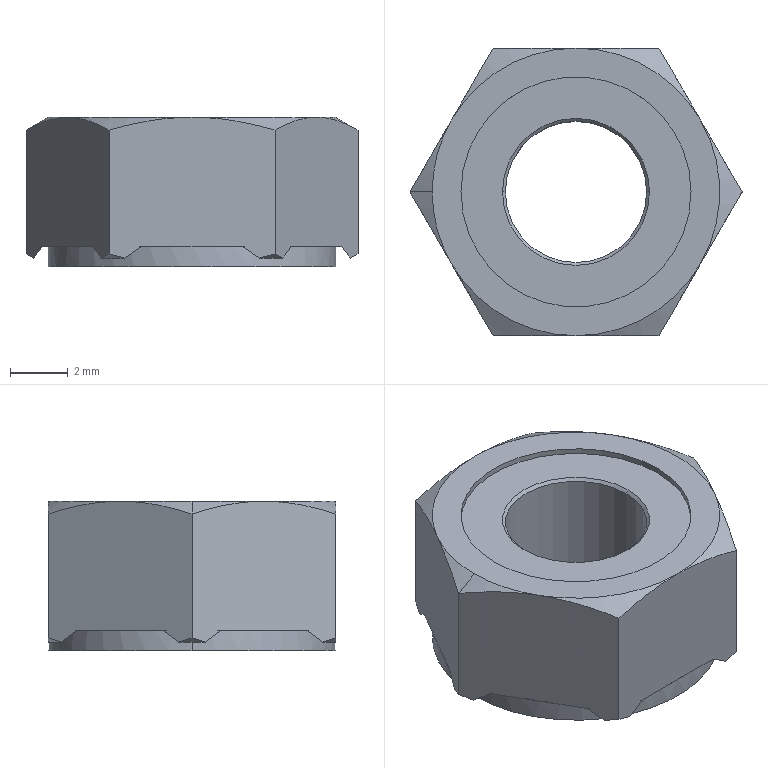Part | STEP file | M6_GB13681_3_VD-SYL0380DJ1006_1 | 1 solid | 45 faces | box 11.547 x 10 x 5.2 mm | volume 338.387 mm3 | cone 24 | plane 15 | cylinder 6 | commonest cylinder face diameters 4.917 x2 8 x2 10 x2
STEP:
#1=CARTESIAN_POINT('',(11.547,0.,0.4466));
#2=VERTEX_POINT('',#1);
#3=CARTESIAN_POINT('',(11.279,-0.4643,0.3031));
#4=VERTEX_POINT('',#3);
#5=CARTESIAN_POINT('',(11.547,0.,0.4466));
#6=CARTESIAN_POINT('',(11.517,-0.05158,0.4294));
#7=CARTESIAN_POINT('',(11.458,-0.1547,0.3958));
#8=CARTESIAN_POINT('',(11.368,-0.3095,0.3479));
#9=CARTESIAN_POINT('',(11.309,-0.4127,0.3177));
#10=CARTESIAN_POINT('',(11.279,-0.4643,0.3031));
#11=B_SPLINE_CURVE_WITH_KNOTS('',3,(#5,#6,#7,#8,#9,#10),.UNSPECIFIED.,.F.,.F.,(4,1,1,4),(0.,0.3333,0.6667,1.),.UNSPECIFIED.);
#12=EDGE_CURVE('',#2,#4,#11,.T.);
#13=ORIENTED_EDGE('',*,*,#12,.T.);
#14=CARTESIAN_POINT('',(11.279,0.4643,0.3031));
#15=VERTEX_POINT('',#14);
#16=CARTESIAN_POINT('',(5.774,0.,0.3031));
#17=DIRECTION('',(0.,0.,1.));
#18=DIRECTION('',(0.9965,-0.08403,0.));
#19=AXIS2_PLACEMENT_3D('',#16,#17,#18);
#20=CIRCLE('',#19,5.525);
#21=EDGE_CURVE('',#4,#15,#20,.T.);
#22=ORIENTED_EDGE('',*,*,#21,.T.);
#23=CARTESIAN_POINT('',(11.279,0.4643,0.3031));
#24=CARTESIAN_POINT('',(11.309,0.4127,0.3177));
#25=CARTESIAN_POINT('',(11.368,0.3095,0.3479));
#26=CARTESIAN_POINT('',(11.458,0.1547,0.3958));
#27=CARTESIAN_POINT('',(11.517,0.05158,0.4294));
#28=CARTESIAN_POINT('',(11.547,0.,0.4466));
#29=B_SPLINE_CURVE_WITH_KNOTS('',3,(#23,#24,#25,#26,#27,#28),.UNSPECIFIED.,.F.,.F.,(4,1,1,4),(0.,0.3333,0.6667,1.),.UNSPECIFIED.);
#30=EDGE_CURVE('',#15,#2,#29,.T.);
#31=ORIENTED_EDGE('',*,*,#30,.T.);
#32=EDGE_LOOP('',(#13,#22,#31));
#33=FACE_OUTER_BOUND('',#32,.T.);
#34=CARTESIAN_POINT('',(5.774,0.,0.3748));
#35=DIRECTION('',(0.,0.,1.));
#36=DIRECTION('',(0.,-1.,0.));
#37=AXIS2_PLACEMENT_3D('',#34,#35,#36);
#38=CONICAL_SURFACE('',#37,5.649,1.047);
#39=ADVANCED_FACE('',(#33),#38,.T.);
#40=CARTESIAN_POINT('',(2.887,5.,0.4466));
#41=VERTEX_POINT('',#40);
#42=CARTESIAN_POINT('',(3.423,5.,0.3031));
#43=VERTEX_POINT('',#42);
#44=CARTESIAN_POINT('',(2.887,5.,0.4466));
#45=CARTESIAN_POINT('',(2.946,5.,0.4294));
#46=CARTESIAN_POINT('',(3.065,5.,0.3958));
#47=CARTESIAN_POINT('',(3.244,5.,0.3479));
#48=CARTESIAN_POINT('',(3.363,5.,0.3177));
#49=CARTESIAN_POINT('',(3.423,5.,0.3031));
#50=B_SPLINE_CURVE_WITH_KNOTS('',3,(#44,#45,#46,#47,#48,#49),.UNSPECIFIED.,.F.,.F.,(4,1,1,4),(0.,0.3333,0.6667,1.),.UNSPECIFIED.);
#51=EDGE_CURVE('',#41,#43,#50,.T.);
#52=ORIENTED_EDGE('',*,*,#51,.T.);
#53=CARTESIAN_POINT('',(2.619,4.536,0.3031));
#54=VERTEX_POINT('',#53);
#55=CARTESIAN_POINT('',(5.774,0.,0.3031));
#56=DIRECTION('',(0.,0.,-1.));
#57=DIRECTION('',(-0.571,0.8209,0.));
#58=AXIS2_PLACEMENT_3D('',#55,#56,#57);
#59=CIRCLE('',#58,5.525);
#60=EDGE_CURVE('',#54,#43,#59,.T.);
#61=ORIENTED_EDGE('',*,*,#60,.F.);
#62=CARTESIAN_POINT('',(2.619,4.536,0.3031));
#63=CARTESIAN_POINT('',(2.648,4.587,0.3177));
#64=CARTESIAN_POINT('',(2.708,4.691,0.3479));
#65=CARTESIAN_POINT('',(2.797,4.845,0.3958));
#66=CARTESIAN_POINT('',(2.857,4.948,0.4294));
#67=CARTESIAN_POINT('',(2.887,5.,0.4466));
#68=B_SPLINE_CURVE_WITH_KNOTS('',3,(#62,#63,#64,#65,#66,#67),.UNSPECIFIED.,.F.,.F.,(4,1,1,4),(0.,0.3333,0.6667,1.),.UNSPECIFIED.);
#69=EDGE_CURVE('',#54,#41,#68,.T.);
#70=ORIENTED_EDGE('',*,*,#69,.T.);
#71=EDGE_LOOP('',(#52,#61,#70));
#72=FACE_OUTER_BOUND('',#71,.T.);
#73=CARTESIAN_POINT('',(5.774,0.,0.3748));
#74=DIRECTION('',(0.,0.,1.));
#75=DIRECTION('',(0.,-1.,0.));
#76=AXIS2_PLACEMENT_3D('',#73,#74,#75);
#77=CONICAL_SURFACE('',#76,5.649,1.047);
#78=ADVANCED_FACE('',(#72),#77,.T.);
#79=CARTESIAN_POINT('',(5.774,5.,0.7));
#80=VERTEX_POINT('',#79);
#81=CARTESIAN_POINT('',(4.028,5.,0.7));
#82=VERTEX_POINT('',#81);
#83=CARTESIAN_POINT('',(5.774,5.,0.7));
#84=DIRECTION('',(-1.,0.,0.));
#85=VECTOR('',#84,1000.);
#86=LINE('',#83,#85);
#87=EDGE_CURVE('',#80,#82,#86,.T.);
#88=ORIENTED_EDGE('',*,*,#87,.F.);
#89=CARTESIAN_POINT('',(1.443,2.5,0.7));
#90=VERTEX_POINT('',#89);
#91=CARTESIAN_POINT('',(5.774,0.,0.7));
#92=DIRECTION('',(0.,0.,1.));
#93=DIRECTION('',(0.,1.,0.));
#94=AXIS2_PLACEMENT_3D('',#91,#92,#93);
#95=CIRCLE('',#94,5.);
#96=EDGE_CURVE('',#80,#90,#95,.T.);
#97=ORIENTED_EDGE('',*,*,#96,.T.);
#98=CARTESIAN_POINT('',(2.316,4.011,0.7));
#99=VERTEX_POINT('',#98);
#100=CARTESIAN_POINT('',(1.443,2.5,0.7));
#101=DIRECTION('',(0.5,0.866,0.));
#102=VECTOR('',#101,1000.);
#103=LINE('',#100,#102);
#104=EDGE_CURVE('',#90,#99,#103,.T.);
#105=ORIENTED_EDGE('',*,*,#104,.T.);
#106=CARTESIAN_POINT('',(5.774,0.,0.7));
#107=DIRECTION('',(0.,0.,-1.));
#108=DIRECTION('',(-0.6529,0.7575,0.));
#109=AXIS2_PLACEMENT_3D('',#106,#107,#108);
#110=CIRCLE('',#109,5.296);
#111=EDGE_CURVE('',#99,#82,#110,.T.);
#112=ORIENTED_EDGE('',*,*,#111,.T.);
#113=EDGE_LOOP('',(#88,#97,#105,#112));
#114=FACE_OUTER_BOUND('',#113,.T.);
#115=CARTESIAN_POINT('',(5.774,0.,0.7));
#116=DIRECTION('',(0.,0.,-1.));
#117=DIRECTION('',(0.,-1.,0.));
#118=AXIS2_PLACEMENT_3D('',#115,#116,#117);
#119=PLANE('',#118);
#120=ADVANCED_FACE('',(#114),#119,.T.);
#121=CARTESIAN_POINT('',(2.887,-5.,0.4466));
#122=VERTEX_POINT('',#121);
#123=CARTESIAN_POINT('',(2.619,-4.536,0.3031));
#124=VERTEX_POINT('',#123);
#125=CARTESIAN_POINT('',(2.887,-5.,0.4466));
#126=CARTESIAN_POINT('',(2.857,-4.948,0.4294));
#127=CARTESIAN_POINT('',(2.797,-4.845,0.3958));
#128=CARTESIAN_POINT('',(2.708,-4.691,0.3479));
#129=CARTESIAN_POINT('',(2.648,-4.587,0.3177));
#130=CARTESIAN_POINT('',(2.619,-4.536,0.3031));
#131=B_SPLINE_CURVE_WITH_KNOTS('',3,(#125,#126,#127,#128,#129,#130),.UNSPECIFIED.,.F.,.F.,(4,1,1,4),(0.,0.3333,0.6667,1.),.UNSPECIFIED.);
#132=EDGE_CURVE('',#122,#124,#131,.T.);
#133=ORIENTED_EDGE('',*,*,#132,.T.);
#134=CARTESIAN_POINT('',(3.423,-5.,0.3031));
#135=VERTEX_POINT('',#134);
#136=CARTESIAN_POINT('',(5.774,0.,0.3031));
#137=DIRECTION('',(0.,0.,-1.));
#138=DIRECTION('',(-0.4255,-0.905,0.));
#139=AXIS2_PLACEMENT_3D('',#136,#137,#138);
#140=CIRCLE('',#139,5.525);
#141=EDGE_CURVE('',#135,#124,#140,.T.);
#142=ORIENTED_EDGE('',*,*,#141,.F.);
#143=CARTESIAN_POINT('',(3.423,-5.,0.3031));
#144=CARTESIAN_POINT('',(3.363,-5.,0.3177));
#145=CARTESIAN_POINT('',(3.244,-5.,0.3479));
#146=CARTESIAN_POINT('',(3.065,-5.,0.3958));
#147=CARTESIAN_POINT('',(2.946,-5.,0.4294));
#148=CARTESIAN_POINT('',(2.887,-5.,0.4466));
#149=B_SPLINE_CURVE_WITH_KNOTS('',3,(#143,#144,#145,#146,#147,#148),.UNSPECIFIED.,.F.,.F.,(4,1,1,4),(0.,0.3333,0.6667,1.),.UNSPECIFIED.);
#150=EDGE_CURVE('',#135,#122,#149,.T.);
#151=ORIENTED_EDGE('',*,*,#150,.T.);
#152=EDGE_LOOP('',(#133,#142,#151));
#153=FACE_OUTER_BOUND('',#152,.T.);
#154=CARTESIAN_POINT('',(5.774,0.,0.3748));
#155=DIRECTION('',(0.,0.,1.));
#156=DIRECTION('',(0.,-1.,0.));
#157=AXIS2_PLACEMENT_3D('',#154,#155,#156);
#158=CONICAL_SURFACE('',#157,5.649,1.047);
#159=ADVANCED_FACE('',(#153),#158,.T.);
#160=CARTESIAN_POINT('',(8.66,-5.,0.4466));
#161=VERTEX_POINT('',#160);
#162=CARTESIAN_POINT('',(8.124,-5.,0.3031));
#163=VERTEX_POINT('',#162);
#164=CARTESIAN_POINT('',(8.66,-5.,0.4466));
#165=CARTESIAN_POINT('',(8.601,-5.,0.4294));
#166=CARTESIAN_POINT('',(8.482,-5.,0.3958));
#167=CARTESIAN_POINT('',(8.303,-5.,0.3479));
#168=CARTESIAN_POINT('',(8.184,-5.,0.3177));
#169=CARTESIAN_POINT('',(8.124,-5.,0.3031));
#170=B_SPLINE_CURVE_WITH_KNOTS('',3,(#164,#165,#166,#167,#168,#169),.UNSPECIFIED.,.F.,.F.,(4,1,1,4),(0.,0.3333,0.6667,1.),.UNSPECIFIED.);
#171=EDGE_CURVE('',#161,#163,#170,.T.);
#172=ORIENTED_EDGE('',*,*,#171,.T.);
#173=CARTESIAN_POINT('',(8.928,-4.536,0.3031));
#174=VERTEX_POINT('',#173);
#175=CARTESIAN_POINT('',(5.774,0.,0.3031));
#176=DIRECTION('',(0.,0.,-1.));
#177=DIRECTION('',(0.571,-0.8209,0.));
#178=AXIS2_PLACEMENT_3D('',#175,#176,#177);
#179=CIRCLE('',#178,5.525);
#180=EDGE_CURVE('',#174,#163,#179,.T.);
#181=ORIENTED_EDGE('',*,*,#180,.F.);
#182=CARTESIAN_POINT('',(8.928,-4.536,0.3031));
#183=CARTESIAN_POINT('',(8.899,-4.587,0.3177));
#184=CARTESIAN_POINT('',(8.839,-4.691,0.3479));
#185=CARTESIAN_POINT('',(8.75,-4.845,0.3958));
#186=CARTESIAN_POINT('',(8.69,-4.948,0.4294));
#187=CARTESIAN_POINT('',(8.66,-5.,0.4466));
#188=B_SPLINE_CURVE_WITH_KNOTS('',3,(#182,#183,#184,#185,#186,#187),.UNSPECIFIED.,.F.,.F.,(4,1,1,4),(0.,0.3333,0.6667,1.),.UNSPECIFIED.);
#189=EDGE_CURVE('',#174,#161,#188,.T.);
#190=ORIENTED_EDGE('',*,*,#189,.T.);
#191=EDGE_LOOP('',(#172,#181,#190));
#192=FACE_OUTER_BOUND('',#191,.T.);
#193=CARTESIAN_POINT('',(5.774,0.,0.3748));
#194=DIRECTION('',(0.,0.,1.));
#195=DIRECTION('',(0.,-1.,0.));
#196=AXIS2_PLACEMENT_3D('',#193,#194,#195);
#197=CONICAL_SURFACE('',#196,5.649,1.047);
#198=ADVANCED_FACE('',(#192),#197,.T.);
#199=CARTESIAN_POINT('',(2.316,-4.011,0.7));
#200=VERTEX_POINT('',#199);
#201=CARTESIAN_POINT('',(1.443,-2.5,0.7));
#202=VERTEX_POINT('',#201);
#203=CARTESIAN_POINT('',(2.316,-4.011,0.7));
#204=DIRECTION('',(-0.5,0.866,0.));
#205=VECTOR('',#204,1000.);
#206=LINE('',#203,#205);
#207=EDGE_CURVE('',#200,#202,#206,.T.);
#208=ORIENTED_EDGE('',*,*,#207,.T.);
#209=CARTESIAN_POINT('',(5.774,-5.,0.7));
#210=VERTEX_POINT('',#209);
#211=CARTESIAN_POINT('',(5.774,0.,0.7));
#212=DIRECTION('',(0.,0.,1.));
#213=DIRECTION('',(-0.866,-0.5,0.));
#214=AXIS2_PLACEMENT_3D('',#211,#212,#213);
#215=CIRCLE('',#214,5.);
#216=EDGE_CURVE('',#202,#210,#215,.T.);
#217=ORIENTED_EDGE('',*,*,#216,.T.);
#218=CARTESIAN_POINT('',(4.028,-5.,0.7));
#219=VERTEX_POINT('',#218);
#220=CARTESIAN_POINT('',(4.028,-5.,0.7));
#221=DIRECTION('',(1.,0.,0.));
#222=VECTOR('',#221,1000.);
#223=LINE('',#220,#222);
#224=EDGE_CURVE('',#219,#210,#223,.T.);
#225=ORIENTED_EDGE('',*,*,#224,.F.);
#226=CARTESIAN_POINT('',(5.774,0.,0.7));
#227=DIRECTION('',(0.,0.,-1.));
#228=DIRECTION('',(-0.3296,-0.9441,0.));
#229=AXIS2_PLACEMENT_3D('',#226,#227,#228);
#230=CIRCLE('',#229,5.296);
#231=EDGE_CURVE('',#219,#200,#230,.T.);
#232=ORIENTED_EDGE('',*,*,#231,.T.);
#233=EDGE_LOOP('',(#208,#217,#225,#232));
#234=FACE_OUTER_BOUND('',#233,.T.);
#235=CARTESIAN_POINT('',(5.774,0.,0.7));
#236=DIRECTION('',(0.,0.,-1.));
#237=DIRECTION('',(0.,-1.,0.));
#238=AXIS2_PLACEMENT_3D('',#235,#236,#237);
#239=PLANE('',#238);
#240=ADVANCED_FACE('',(#234),#239,.T.);
#241=CARTESIAN_POINT('',(2.887,-5.,4.753));
#242=VERTEX_POINT('',#241);
#243=CARTESIAN_POINT('',(5.774,-5.,5.2));
#244=VERTEX_POINT('',#243);
#245=CARTESIAN_POINT('',(2.887,-5.,4.753));
#246=CARTESIAN_POINT('',(3.393,-5.,4.9));
#247=CARTESIAN_POINT('',(3.874,-5.,5.01));
#248=CARTESIAN_POINT('',(4.838,-5.,5.162));
#249=CARTESIAN_POINT('',(5.299,-5.,5.2));
#250=CARTESIAN_POINT('',(5.774,-5.,5.2));
#251=B_SPLINE_CURVE_WITH_KNOTS('',3,(#245,#246,#247,#248,#249,#250),.UNSPECIFIED.,.F.,.F.,(4,2,4),(0.,0.5,1.),.UNSPECIFIED.);
#252=EDGE_CURVE('',#242,#244,#251,.T.);
#253=ORIENTED_EDGE('',*,*,#252,.T.);
#254=CARTESIAN_POINT('',(1.443,-2.5,5.2));
#255=VERTEX_POINT('',#254);
#256=CARTESIAN_POINT('',(5.774,0.,5.2));
#257=DIRECTION('',(0.,0.,1.));
#258=DIRECTION('',(-0.866,-0.5,0.));
#259=AXIS2_PLACEMENT_3D('',#256,#257,#258);
#260=CIRCLE('',#259,5.);
#261=EDGE_CURVE('',#255,#244,#260,.T.);
#262=ORIENTED_EDGE('',*,*,#261,.F.);
#263=CARTESIAN_POINT('',(1.443,-2.5,5.2));
#264=CARTESIAN_POINT('',(1.562,-2.706,5.2));
#265=CARTESIAN_POINT('',(1.679,-2.908,5.19));
#266=CARTESIAN_POINT('',(1.914,-3.315,5.152));
#267=CARTESIAN_POINT('',(2.033,-3.521,5.124));
#268=CARTESIAN_POINT('',(2.393,-4.145,5.01));
#269=CARTESIAN_POINT('',(2.634,-4.562,4.899));
#270=CARTESIAN_POINT('',(2.887,-5.,4.753));
#271=B_SPLINE_CURVE_WITH_KNOTS('',3,(#263,#264,#265,#266,#267,#268,#269,#270),.UNSPECIFIED.,.F.,.F.,(4,2,2,4),(0.,0.25,0.5,1.),.UNSPECIFIED.);
#272=EDGE_CURVE('',#255,#242,#271,.T.);
#273=ORIENTED_EDGE('',*,*,#272,.T.);
#274=EDGE_LOOP('',(#253,#262,#273));
#275=FACE_OUTER_BOUND('',#274,.T.);
#276=CARTESIAN_POINT('',(5.774,0.,4.977));
#277=DIRECTION('',(0.,0.,-1.));
#278=DIRECTION('',(-1.,0.,0.));
#279=AXIS2_PLACEMENT_3D('',#276,#277,#278);
#280=CONICAL_SURFACE('',#279,5.387,1.047);
#281=ADVANCED_FACE('',(#275),#280,.T.);
#282=CARTESIAN_POINT('',(8.66,-5.,4.753));
#283=VERTEX_POINT('',#282);
#284=CARTESIAN_POINT('',(10.104,-2.5,5.2));
#285=VERTEX_POINT('',#284);
#286=CARTESIAN_POINT('',(8.66,-5.,4.753));
#287=CARTESIAN_POINT('',(8.913,-4.562,4.9));
#288=CARTESIAN_POINT('',(9.154,-4.145,5.01));
#289=CARTESIAN_POINT('',(9.636,-3.31,5.162));
#290=CARTESIAN_POINT('',(9.866,-2.911,5.2));
#291=CARTESIAN_POINT('',(10.104,-2.5,5.2));
#292=B_SPLINE_CURVE_WITH_KNOTS('',3,(#286,#287,#288,#289,#290,#291),.UNSPECIFIED.,.F.,.F.,(4,2,4),(0.,0.5,1.),.UNSPECIFIED.);
#293=EDGE_CURVE('',#283,#285,#292,.T.);
#294=ORIENTED_EDGE('',*,*,#293,.T.);
#295=CARTESIAN_POINT('',(5.774,0.,5.2));
#296=DIRECTION('',(0.,0.,1.));
#297=DIRECTION('',(0.,-1.,0.));
#298=AXIS2_PLACEMENT_3D('',#295,#296,#297);
#299=CIRCLE('',#298,5.);
#300=EDGE_CURVE('',#244,#285,#299,.T.);
#301=ORIENTED_EDGE('',*,*,#300,.F.);
#302=CARTESIAN_POINT('',(5.774,-5.,5.2));
#303=CARTESIAN_POINT('',(6.011,-5.,5.2));
#304=CARTESIAN_POINT('',(6.245,-5.,5.19));
#305=CARTESIAN_POINT('',(6.715,-5.,5.152));
#306=CARTESIAN_POINT('',(6.952,-5.,5.124));
#307=CARTESIAN_POINT('',(7.672,-5.,5.01));
#308=CARTESIAN_POINT('',(8.154,-5.,4.899));
#309=CARTESIAN_POINT('',(8.66,-5.,4.753));
#310=B_SPLINE_CURVE_WITH_KNOTS('',3,(#302,#303,#304,#305,#306,#307,#308,#309),.UNSPECIFIED.,.F.,.F.,(4,2,2,4),(0.,0.25,0.5,1.),.UNSPECIFIED.);
#311=EDGE_CURVE('',#244,#283,#310,.T.);
#312=ORIENTED_EDGE('',*,*,#311,.T.);
#313=EDGE_LOOP('',(#294,#301,#312));
#314=FACE_OUTER_BOUND('',#313,.T.);
#315=CARTESIAN_POINT('',(5.774,0.,4.977));
#316=DIRECTION('',(0.,0.,-1.));
#317=DIRECTION('',(-1.,0.,0.));
#318=AXIS2_PLACEMENT_3D('',#315,#316,#317);
#319=CONICAL_SURFACE('',#318,5.387,1.047);
#320=ADVANCED_FACE('',(#314),#319,.T.);
#321=CARTESIAN_POINT('',(11.547,0.,4.753));
#322=VERTEX_POINT('',#321);
#323=CARTESIAN_POINT('',(10.104,2.5,5.2));
#324=VERTEX_POINT('',#323);
#325=CARTESIAN_POINT('',(11.547,0.,4.753));
#326=CARTESIAN_POINT('',(11.294,0.4384,4.9));
#327=CARTESIAN_POINT('',(11.053,0.8554,5.01));
#328=CARTESIAN_POINT('',(10.571,1.69,5.162));
#329=CARTESIAN_POINT('',(10.341,2.089,5.2));
#330=CARTESIAN_POINT('',(10.104,2.5,5.2));
#331=B_SPLINE_CURVE_WITH_KNOTS('',3,(#325,#326,#327,#328,#329,#330),.UNSPECIFIED.,.F.,.F.,(4,2,4),(0.,0.5,1.),.UNSPECIFIED.);
#332=EDGE_CURVE('',#322,#324,#331,.T.);
#333=ORIENTED_EDGE('',*,*,#332,.T.);
#334=CARTESIAN_POINT('',(5.774,0.,5.2));
#335=DIRECTION('',(0.,0.,1.));
#336=DIRECTION('',(0.866,-0.5,0.));
#337=AXIS2_PLACEMENT_3D('',#334,#335,#336);
#338=CIRCLE('',#337,5.);
#339=EDGE_CURVE('',#285,#324,#338,.T.);
#340=ORIENTED_EDGE('',*,*,#339,.F.);
#341=CARTESIAN_POINT('',(10.104,-2.5,5.2));
#342=CARTESIAN_POINT('',(10.222,-2.294,5.2));
#343=CARTESIAN_POINT('',(10.339,-2.092,5.19));
#344=CARTESIAN_POINT('',(10.574,-1.685,5.152));
#345=CARTESIAN_POINT('',(10.693,-1.479,5.124));
#346=CARTESIAN_POINT('',(11.053,-0.8555,5.01));
#347=CARTESIAN_POINT('',(11.294,-0.438,4.899));
#348=CARTESIAN_POINT('',(11.547,0.,4.753));
#349=B_SPLINE_CURVE_WITH_KNOTS('',3,(#341,#342,#343,#344,#345,#346,#347,#348),.UNSPECIFIED.,.F.,.F.,(4,2,2,4),(0.,0.25,0.5,1.),.UNSPECIFIED.);
#350=EDGE_CURVE('',#285,#322,#349,.T.);
#351=ORIENTED_EDGE('',*,*,#350,.T.);
#352=EDGE_LOOP('',(#333,#340,#351));
#353=FACE_OUTER_BOUND('',#352,.T.);
#354=CARTESIAN_POINT('',(5.774,0.,4.977));
#355=DIRECTION('',(0.,0.,-1.));
#356=DIRECTION('',(-1.,0.,0.));
#357=AXIS2_PLACEMENT_3D('',#354,#355,#356);
#358=CONICAL_SURFACE('',#357,5.387,1.047);
#359=ADVANCED_FACE('',(#353),#358,.T.);
#360=CARTESIAN_POINT('',(8.66,5.,4.753));
#361=VERTEX_POINT('',#360);
#362=CARTESIAN_POINT('',(5.774,5.,5.2));
#363=VERTEX_POINT('',#362);
#364=CARTESIAN_POINT('',(8.66,5.,4.753));
#365=CARTESIAN_POINT('',(8.154,5.,4.9));
#366=CARTESIAN_POINT('',(7.673,5.,5.01));
#367=CARTESIAN_POINT('',(6.709,5.,5.162));
#368=CARTESIAN_POINT('',(6.248,5.,5.2));
#369=CARTESIAN_POINT('',(5.774,5.,5.2));
#370=B_SPLINE_CURVE_WITH_KNOTS('',3,(#364,#365,#366,#367,#368,#369),.UNSPECIFIED.,.F.,.F.,(4,2,4),(0.,0.5,1.),.UNSPECIFIED.);
#371=EDGE_CURVE('',#361,#363,#370,.T.);
#372=ORIENTED_EDGE('',*,*,#371,.T.);
#373=CARTESIAN_POINT('',(5.774,0.,5.2));
#374=DIRECTION('',(0.,0.,1.));
#375=DIRECTION('',(0.866,0.5,0.));
#376=AXIS2_PLACEMENT_3D('',#373,#374,#375);
#377=CIRCLE('',#376,5.);
#378=EDGE_CURVE('',#324,#363,#377,.T.);
#379=ORIENTED_EDGE('',*,*,#378,.F.);
#380=CARTESIAN_POINT('',(10.104,2.5,5.2));
#381=CARTESIAN_POINT('',(9.985,2.706,5.2));
#382=CARTESIAN_POINT('',(9.868,2.908,5.19));
#383=CARTESIAN_POINT('',(9.633,3.315,5.152));
#384=CARTESIAN_POINT('',(9.514,3.521,5.124));
#385=CARTESIAN_POINT('',(9.154,4.145,5.01));
#386=CARTESIAN_POINT('',(8.913,4.562,4.899));
#387=CARTESIAN_POINT('',(8.66,5.,4.753));
#388=B_SPLINE_CURVE_WITH_KNOTS('',3,(#380,#381,#382,#383,#384,#385,#386,#387),.UNSPECIFIED.,.F.,.F.,(4,2,2,4),(0.,0.25,0.5,1.),.UNSPECIFIED.);
#389=EDGE_CURVE('',#324,#361,#388,.T.);
#390=ORIENTED_EDGE('',*,*,#389,.T.);
#391=EDGE_LOOP('',(#372,#379,#390));
#392=FACE_OUTER_BOUND('',#391,.T.);
#393=CARTESIAN_POINT('',(5.774,0.,4.977));
#394=DIRECTION('',(0.,0.,-1.));
#395=DIRECTION('',(-1.,0.,0.));
#396=AXIS2_PLACEMENT_3D('',#393,#394,#395);
#397=CONICAL_SURFACE('',#396,5.387,1.047);
#398=ADVANCED_FACE('',(#392),#397,.T.);
#399=CARTESIAN_POINT('',(2.887,5.,4.753));
#400=VERTEX_POINT('',#399);
#401=CARTESIAN_POINT('',(1.443,2.5,5.2));
#402=VERTEX_POINT('',#401);
#403=CARTESIAN_POINT('',(2.887,5.,4.753));
#404=CARTESIAN_POINT('',(2.634,4.562,4.9));
#405=CARTESIAN_POINT('',(2.393,4.145,5.01));
#406=CARTESIAN_POINT('',(1.911,3.31,5.162));
#407=CARTESIAN_POINT('',(1.681,2.911,5.2));
#408=CARTESIAN_POINT('',(1.443,2.5,5.2));
#409=B_SPLINE_CURVE_WITH_KNOTS('',3,(#403,#404,#405,#406,#407,#408),.UNSPECIFIED.,.F.,.F.,(4,2,4),(0.,0.5,1.),.UNSPECIFIED.);
#410=EDGE_CURVE('',#400,#402,#409,.T.);
#411=ORIENTED_EDGE('',*,*,#410,.T.);
#412=CARTESIAN_POINT('',(5.774,0.,5.2));
#413=DIRECTION('',(0.,0.,1.));
#414=DIRECTION('',(0.000000019,1.,0.));
#415=AXIS2_PLACEMENT_3D('',#412,#413,#414);
#416=CIRCLE('',#415,5.);
#417=EDGE_CURVE('',#363,#402,#416,.T.);
#418=ORIENTED_EDGE('',*,*,#417,.F.);
#419=CARTESIAN_POINT('',(5.774,5.,5.2));
#420=CARTESIAN_POINT('',(5.536,5.,5.2));
#421=CARTESIAN_POINT('',(5.302,5.,5.19));
#422=CARTESIAN_POINT('',(4.832,5.,5.152));
#423=CARTESIAN_POINT('',(4.595,5.,5.124));
#424=CARTESIAN_POINT('',(3.875,5.,5.01));
#425=CARTESIAN_POINT('',(3.393,5.,4.899));
#426=CARTESIAN_POINT('',(2.887,5.,4.753));
#427=B_SPLINE_CURVE_WITH_KNOTS('',3,(#419,#420,#421,#422,#423,#424,#425,#426),.UNSPECIFIED.,.F.,.F.,(4,2,2,4),(0.,0.25,0.5,1.),.UNSPECIFIED.);
#428=EDGE_CURVE('',#363,#400,#427,.T.);
#429=ORIENTED_EDGE('',*,*,#428,.T.);
#430=EDGE_LOOP('',(#411,#418,#429));
#431=FACE_OUTER_BOUND('',#430,.T.);
#432=CARTESIAN_POINT('',(5.774,0.,4.977));
#433=DIRECTION('',(0.,0.,-1.));
#434=DIRECTION('',(-1.,0.,0.));
#435=AXIS2_PLACEMENT_3D('',#432,#433,#434);
#436=CONICAL_SURFACE('',#435,5.387,1.047);
#437=ADVANCED_FACE('',(#431),#436,.T.);
#438=CARTESIAN_POINT('',(0.7735,0.,5.2));
#439=VERTEX_POINT('',#438);
#440=CARTESIAN_POINT('',(5.774,0.,5.2));
#441=DIRECTION('',(0.,0.,1.));
#442=DIRECTION('',(-0.866,0.5,0.));
#443=AXIS2_PLACEMENT_3D('',#440,#441,#442);
#444=CIRCLE('',#443,5.);
#445=EDGE_CURVE('',#402,#439,#444,.T.);
#446=ORIENTED_EDGE('',*,*,#445,.F.);
#447=CARTESIAN_POINT('',(0.,0.,4.753));
#448=VERTEX_POINT('',#447);
#449=CARTESIAN_POINT('',(1.443,2.5,5.2));
#450=CARTESIAN_POINT('',(1.325,2.294,5.2));
#451=CARTESIAN_POINT('',(1.208,2.092,5.19));
#452=CARTESIAN_POINT('',(0.9728,1.685,5.152));
#453=CARTESIAN_POINT('',(0.8539,1.479,5.124));
#454=CARTESIAN_POINT('',(0.4937,0.8555,5.01));
#455=CARTESIAN_POINT('',(0.2529,0.438,4.899));
#456=CARTESIAN_POINT('',(0.,0.,4.753));
#457=B_SPLINE_CURVE_WITH_KNOTS('',3,(#449,#450,#451,#452,#453,#454,#455,#456),.UNSPECIFIED.,.F.,.F.,(4,2,2,4),(0.,0.25,0.5,1.),.UNSPECIFIED.);
#458=EDGE_CURVE('',#402,#448,#457,.T.);
#459=ORIENTED_EDGE('',*,*,#458,.T.);
#460=CARTESIAN_POINT('',(0.,0.,4.753));
#461=DIRECTION('',(0.866,0.,0.5));
#462=VECTOR('',#461,1000.);
#463=LINE('',#460,#462);
#464=EDGE_CURVE('',#448,#439,#463,.T.);
#465=ORIENTED_EDGE('',*,*,#464,.T.);
#466=EDGE_LOOP('',(#446,#459,#465));
#467=FACE_OUTER_BOUND('',#466,.T.);
#468=CARTESIAN_POINT('',(5.774,0.,4.977));
#469=DIRECTION('',(0.,0.,-1.));
#470=DIRECTION('',(-1.,0.,0.));
#471=AXIS2_PLACEMENT_3D('',#468,#469,#470);
#472=CONICAL_SURFACE('',#471,5.387,1.047);
#473=ADVANCED_FACE('',(#467),#472,.T.);
#474=ORIENTED_EDGE('',*,*,#464,.F.);
#475=CARTESIAN_POINT('',(0.,0.,4.753));
#476=CARTESIAN_POINT('',(0.2531,-0.4384,4.9));
#477=CARTESIAN_POINT('',(0.4936,-0.8554,5.01));
#478=CARTESIAN_POINT('',(0.9756,-1.69,5.162));
#479=CARTESIAN_POINT('',(1.206,-2.089,5.2));
#480=CARTESIAN_POINT('',(1.443,-2.5,5.2));
#481=B_SPLINE_CURVE_WITH_KNOTS('',3,(#475,#476,#477,#478,#479,#480),.UNSPECIFIED.,.F.,.F.,(4,2,4),(0.,0.5,1.),.UNSPECIFIED.);
#482=EDGE_CURVE('',#448,#255,#481,.T.);
#483=ORIENTED_EDGE('',*,*,#482,.T.);
#484=CARTESIAN_POINT('',(5.774,0.,5.2));
#485=DIRECTION('',(0.,0.,1.));
#486=DIRECTION('',(-1.,0.,0.));
#487=AXIS2_PLACEMENT_3D('',#484,#485,#486);
#488=CIRCLE('',#487,5.);
#489=EDGE_CURVE('',#439,#255,#488,.T.);
#490=ORIENTED_EDGE('',*,*,#489,.F.);
#491=EDGE_LOOP('',(#474,#483,#490));
#492=FACE_OUTER_BOUND('',#491,.T.);
#493=CARTESIAN_POINT('',(5.774,0.,4.977));
#494=DIRECTION('',(0.,0.,-1.));
#495=DIRECTION('',(-1.,0.,0.));
#496=AXIS2_PLACEMENT_3D('',#493,#494,#495);
#497=CONICAL_SURFACE('',#496,5.387,1.047);
#498=ADVANCED_FACE('',(#492),#497,.T.);
#499=CARTESIAN_POINT('',(1.774,0.,5.2));
#500=VERTEX_POINT('',#499);
#501=CARTESIAN_POINT('',(9.774,0.,5.2));
#502=VERTEX_POINT('',#501);
#503=CARTESIAN_POINT('',(5.774,0.,5.2));
#504=DIRECTION('',(0.,0.,-1.));
#505=DIRECTION('',(-1.,0.,0.));
#506=AXIS2_PLACEMENT_3D('',#503,#504,#505);
#507=CIRCLE('',#506,4.);
#508=EDGE_CURVE('',#500,#502,#507,.T.);
#509=ORIENTED_EDGE('',*,*,#508,.T.);
#510=CARTESIAN_POINT('',(5.774,0.,5.2));
#511=DIRECTION('',(0.,0.,-1.));
#512=DIRECTION('',(1.,0.,0.));
#513=AXIS2_PLACEMENT_3D('',#510,#511,#512);
#514=CIRCLE('',#513,4.);
#515=EDGE_CURVE('',#502,#500,#514,.T.);
#516=ORIENTED_EDGE('',*,*,#515,.T.);
#517=EDGE_LOOP('',(#509,#516));
#518=FACE_BOUND('',#517,.T.);
#519=ORIENTED_EDGE('',*,*,#261,.T.);
#520=ORIENTED_EDGE('',*,*,#300,.T.);
#521=ORIENTED_EDGE('',*,*,#339,.T.);
#522=ORIENTED_EDGE('',*,*,#378,.T.);
#523=ORIENTED_EDGE('',*,*,#417,.T.);
#524=ORIENTED_EDGE('',*,*,#445,.T.);
#525=ORIENTED_EDGE('',*,*,#489,.T.);
#526=EDGE_LOOP('',(#519,#520,#521,#522,#523,#524,#525));
#527=FACE_OUTER_BOUND('',#526,.T.);
#528=CARTESIAN_POINT('',(0.,0.,5.2));
#529=DIRECTION('',(0.,0.,1.));
#530=DIRECTION('',(1.,0.,0.));
#531=AXIS2_PLACEMENT_3D('',#528,#529,#530);
#532=PLANE('',#531);
#533=ADVANCED_FACE('',(#518,#527),#532,.T.);
#534=CARTESIAN_POINT('',(1.774,0.,5.));
#535=VERTEX_POINT('',#534);
#536=CARTESIAN_POINT('',(1.774,0.,5.2));
#537=DIRECTION('',(0.,0.,-1.));
#538=VECTOR('',#537,1000.);
#539=LINE('',#536,#538);
#540=EDGE_CURVE('',#500,#535,#539,.T.);
#541=ORIENTED_EDGE('',*,*,#540,.F.);
#542=ORIENTED_EDGE('',*,*,#515,.F.);
#543=CARTESIAN_POINT('',(9.774,0.,5.));
#544=VERTEX_POINT('',#543);
#545=CARTESIAN_POINT('',(9.774,0.,5.2));
#546=DIRECTION('',(0.,0.,-1.));
#547=VECTOR('',#546,1000.);
#548=LINE('',#545,#547);
#549=EDGE_CURVE('',#502,#544,#548,.T.);
#550=ORIENTED_EDGE('',*,*,#549,.T.);
#551=CARTESIAN_POINT('',(5.774,0.,5.));
#552=DIRECTION('',(0.,0.,1.));
#553=DIRECTION('',(-1.,0.,0.));
#554=AXIS2_PLACEMENT_3D('',#551,#552,#553);
#555=CIRCLE('',#554,4.);
#556=EDGE_CURVE('',#535,#544,#555,.T.);
#557=ORIENTED_EDGE('',*,*,#556,.F.);
#558=EDGE_LOOP('',(#541,#542,#550,#557));
#559=FACE_OUTER_BOUND('',#558,.T.);
#560=CARTESIAN_POINT('',(5.774,0.,4.99));
#561=DIRECTION('',(0.,0.,1.));
#562=DIRECTION('',(1.,0.,0.));
#563=AXIS2_PLACEMENT_3D('',#560,#561,#562);
#564=CYLINDRICAL_SURFACE('',#563,4.);
#565=ADVANCED_FACE('',(#559),#564,.F.);
#566=CARTESIAN_POINT('',(5.774,0.,5.));
#567=DIRECTION('',(0.,0.,1.));
#568=DIRECTION('',(1.,0.,0.));
#569=AXIS2_PLACEMENT_3D('',#566,#567,#568);
#570=CIRCLE('',#569,4.);
#571=EDGE_CURVE('',#544,#535,#570,.T.);
#572=ORIENTED_EDGE('',*,*,#571,.F.);
#573=ORIENTED_EDGE('',*,*,#549,.F.);
#574=ORIENTED_EDGE('',*,*,#508,.F.);
#575=ORIENTED_EDGE('',*,*,#540,.T.);
#576=EDGE_LOOP('',(#572,#573,#574,#575));
#577=FACE_OUTER_BOUND('',#576,.T.);
#578=CARTESIAN_POINT('',(5.774,0.,4.99));
#579=DIRECTION('',(0.,0.,1.));
#580=DIRECTION('',(1.,0.,0.));
#581=AXIS2_PLACEMENT_3D('',#578,#579,#580);
#582=CYLINDRICAL_SURFACE('',#581,4.);
#583=ADVANCED_FACE('',(#577),#582,.F.);
#584=CARTESIAN_POINT('',(3.215,0.,5.));
#585=VERTEX_POINT('',#584);
#586=CARTESIAN_POINT('',(8.332,0.,5.));
#587=VERTEX_POINT('',#586);
#588=CARTESIAN_POINT('',(5.774,0.,5.));
#589=DIRECTION('',(0.,0.,-1.));
#590=DIRECTION('',(-1.,0.,0.));
#591=AXIS2_PLACEMENT_3D('',#588,#589,#590);
#592=CIRCLE('',#591,2.559);
#593=EDGE_CURVE('',#585,#587,#592,.T.);
#594=ORIENTED_EDGE('',*,*,#593,.T.);
#595=CARTESIAN_POINT('',(5.774,0.,5.));
#596=DIRECTION('',(0.,0.,-1.));
#597=DIRECTION('',(1.,0.,0.));
#598=AXIS2_PLACEMENT_3D('',#595,#596,#597);
#599=CIRCLE('',#598,2.559);
#600=EDGE_CURVE('',#587,#585,#599,.T.);
#601=ORIENTED_EDGE('',*,*,#600,.T.);
#602=EDGE_LOOP('',(#594,#601));
#603=FACE_BOUND('',#602,.T.);
#604=ORIENTED_EDGE('',*,*,#556,.T.);
#605=ORIENTED_EDGE('',*,*,#571,.T.);
#606=EDGE_LOOP('',(#604,#605));
#607=FACE_OUTER_BOUND('',#606,.T.);
#608=CARTESIAN_POINT('',(5.774,0.,5.));
#609=DIRECTION('',(0.,0.,1.));
#610=DIRECTION('',(1.,0.,0.));
#611=AXIS2_PLACEMENT_3D('',#608,#609,#610);
#612=PLANE('',#611);
#613=ADVANCED_FACE('',(#603,#607),#612,.T.);
#614=CARTESIAN_POINT('',(3.315,0.,4.9));
#615=VERTEX_POINT('',#614);
#616=CARTESIAN_POINT('',(3.215,0.,5.));
#617=DIRECTION('',(0.7071,0.,-0.7071));
#618=VECTOR('',#617,1000.);
#619=LINE('',#616,#618);
#620=EDGE_CURVE('',#585,#615,#619,.T.);
#621=ORIENTED_EDGE('',*,*,#620,.F.);
#622=ORIENTED_EDGE('',*,*,#600,.F.);
#623=CARTESIAN_POINT('',(8.232,0.,4.9));
#624=VERTEX_POINT('',#623);
#625=CARTESIAN_POINT('',(8.332,0.,5.));
#626=DIRECTION('',(-0.7071,0.,-0.7071));
#627=VECTOR('',#626,1000.);
#628=LINE('',#625,#627);
#629=EDGE_CURVE('',#587,#624,#628,.T.);
#630=ORIENTED_EDGE('',*,*,#629,.T.);
#631=CARTESIAN_POINT('',(5.774,0.,4.9));
#632=DIRECTION('',(0.,0.,-1.));
#633=DIRECTION('',(1.,0.,0.));
#634=AXIS2_PLACEMENT_3D('',#631,#632,#633);
#635=CIRCLE('',#634,2.458);
#636=EDGE_CURVE('',#624,#615,#635,.T.);
#637=ORIENTED_EDGE('',*,*,#636,.T.);
#638=EDGE_LOOP('',(#621,#622,#630,#637));
#639=FACE_OUTER_BOUND('',#638,.T.);
#640=CARTESIAN_POINT('',(5.774,0.,4.95));
#641=DIRECTION('',(0.,0.,1.));
#642=DIRECTION('',(1.,0.,0.));
#643=AXIS2_PLACEMENT_3D('',#640,#641,#642);
#644=CONICAL_SURFACE('',#643,2.509,0.7854);
#645=ADVANCED_FACE('',(#639),#644,.F.);
#646=CARTESIAN_POINT('',(5.774,0.,4.9));
#647=DIRECTION('',(0.,0.,-1.));
#648=DIRECTION('',(-1.,0.,0.));
#649=AXIS2_PLACEMENT_3D('',#646,#647,#648);
#650=CIRCLE('',#649,2.458);
#651=EDGE_CURVE('',#615,#624,#650,.T.);
#652=ORIENTED_EDGE('',*,*,#651,.T.);
#653=ORIENTED_EDGE('',*,*,#629,.F.);
#654=ORIENTED_EDGE('',*,*,#593,.F.);
#655=ORIENTED_EDGE('',*,*,#620,.T.);
#656=EDGE_LOOP('',(#652,#653,#654,#655));
#657=FACE_OUTER_BOUND('',#656,.T.);
#658=CARTESIAN_POINT('',(5.774,0.,4.95));
#659=DIRECTION('',(0.,0.,1.));
#660=DIRECTION('',(1.,0.,0.));
#661=AXIS2_PLACEMENT_3D('',#658,#659,#660);
#662=CONICAL_SURFACE('',#661,2.509,0.7854);
#663=ADVANCED_FACE('',(#657),#662,.F.);
#664=CARTESIAN_POINT('',(8.232,0.,0.3));
#665=VERTEX_POINT('',#664);
#666=CARTESIAN_POINT('',(3.315,0.,0.3));
#667=VERTEX_POINT('',#666);
#668=CARTESIAN_POINT('',(5.774,0.,0.3));
#669=DIRECTION('',(0.,0.,1.));
#670=DIRECTION('',(1.,0.,0.));
#671=AXIS2_PLACEMENT_3D('',#668,#669,#670);
#672=CIRCLE('',#671,2.459);
#673=EDGE_CURVE('',#665,#667,#672,.T.);
#674=ORIENTED_EDGE('',*,*,#673,.F.);
#675=CARTESIAN_POINT('',(8.232,0.,4.9));
#676=DIRECTION('',(0.,0.,-1.));
#677=VECTOR('',#676,1000.);
#678=LINE('',#675,#677);
#679=EDGE_CURVE('',#624,#665,#678,.T.);
#680=ORIENTED_EDGE('',*,*,#679,.F.);
#681=ORIENTED_EDGE('',*,*,#651,.F.);
#682=CARTESIAN_POINT('',(3.315,0.,4.9));
#683=DIRECTION('',(0.,0.,-1.));
#684=VECTOR('',#683,1000.);
#685=LINE('',#682,#684);
#686=EDGE_CURVE('',#615,#667,#685,.T.);
#687=ORIENTED_EDGE('',*,*,#686,.T.);
#688=EDGE_LOOP('',(#674,#680,#681,#687));
#689=FACE_OUTER_BOUND('',#688,.T.);
#690=CARTESIAN_POINT('',(5.774,0.,0.));
#691=DIRECTION('',(0.,0.,1.));
#692=DIRECTION('',(1.,0.,0.));
#693=AXIS2_PLACEMENT_3D('',#690,#691,#692);
#694=CYLINDRICAL_SURFACE('',#693,2.458);
#695=ADVANCED_FACE('',(#689),#694,.F.);
#696=ORIENTED_EDGE('',*,*,#686,.F.);
#697=ORIENTED_EDGE('',*,*,#636,.F.);
#698=ORIENTED_EDGE('',*,*,#679,.T.);
#699=CARTESIAN_POINT('',(5.774,0.,0.3));
#700=DIRECTION('',(0.,0.,1.));
#701=DIRECTION('',(-1.,0.,0.));
#702=AXIS2_PLACEMENT_3D('',#699,#700,#701);
#703=CIRCLE('',#702,2.459);
#704=EDGE_CURVE('',#667,#665,#703,.T.);
#705=ORIENTED_EDGE('',*,*,#704,.F.);
#706=EDGE_LOOP('',(#696,#697,#698,#705));
#707=FACE_OUTER_BOUND('',#706,.T.);
#708=CARTESIAN_POINT('',(5.774,0.,0.));
#709=DIRECTION('',(0.,0.,1.));
#710=DIRECTION('',(1.,0.,0.));
#711=AXIS2_PLACEMENT_3D('',#708,#709,#710);
#712=CYLINDRICAL_SURFACE('',#711,2.458);
#713=ADVANCED_FACE('',(#707),#712,.F.);
#714=CARTESIAN_POINT('',(8.532,0.,0.));
#715=VERTEX_POINT('',#714);
#716=CARTESIAN_POINT('',(8.532,0.,0.));
#717=DIRECTION('',(-0.7071,0.,0.7071));
#718=VECTOR('',#717,1000.);
#719=LINE('',#716,#718);
#720=EDGE_CURVE('',#715,#665,#719,.T.);
#721=ORIENTED_EDGE('',*,*,#720,.F.);
#722=CARTESIAN_POINT('',(3.015,0.,0.));
#723=VERTEX_POINT('',#722);
#724=CARTESIAN_POINT('',(5.774,0.,0.));
#725=DIRECTION('',(0.,0.,1.));
#726=DIRECTION('',(-1.,0.,0.));
#727=AXIS2_PLACEMENT_3D('',#724,#725,#726);
#728=CIRCLE('',#727,2.759);
#729=EDGE_CURVE('',#723,#715,#728,.T.);
#730=ORIENTED_EDGE('',*,*,#729,.F.);
#731=CARTESIAN_POINT('',(3.015,0.,0.));
#732=DIRECTION('',(0.7071,0.,0.7071));
#733=VECTOR('',#732,1000.);
#734=LINE('',#731,#733);
#735=EDGE_CURVE('',#723,#667,#734,.T.);
#736=ORIENTED_EDGE('',*,*,#735,.T.);
#737=ORIENTED_EDGE('',*,*,#704,.T.);
#738=EDGE_LOOP('',(#721,#730,#736,#737));
#739=FACE_OUTER_BOUND('',#738,.T.);
#740=CARTESIAN_POINT('',(5.774,0.,0.15));
#741=DIRECTION('',(0.,0.,-1.));
#742=DIRECTION('',(-1.,0.,0.));
#743=AXIS2_PLACEMENT_3D('',#740,#741,#742);
#744=CONICAL_SURFACE('',#743,2.609,0.7854);
#745=ADVANCED_FACE('',(#739),#744,.F.);
#746=ORIENTED_EDGE('',*,*,#673,.T.);
#747=ORIENTED_EDGE('',*,*,#735,.F.);
#748=CARTESIAN_POINT('',(5.774,0.,0.));
#749=DIRECTION('',(0.,0.,1.));
#750=DIRECTION('',(1.,0.,0.));
#751=AXIS2_PLACEMENT_3D('',#748,#749,#750);
#752=CIRCLE('',#751,2.759);
#753=EDGE_CURVE('',#715,#723,#752,.T.);
#754=ORIENTED_EDGE('',*,*,#753,.F.);
#755=ORIENTED_EDGE('',*,*,#720,.T.);
#756=EDGE_LOOP('',(#746,#747,#754,#755));
#757=FACE_OUTER_BOUND('',#756,.T.);
#758=CARTESIAN_POINT('',(5.774,0.,0.15));
#759=DIRECTION('',(0.,0.,-1.));
#760=DIRECTION('',(-1.,0.,0.));
#761=AXIS2_PLACEMENT_3D('',#758,#759,#760);
#762=CONICAL_SURFACE('',#761,2.609,0.7854);
#763=ADVANCED_FACE('',(#757),#762,.F.);
#764=ORIENTED_EDGE('',*,*,#729,.T.);
#765=ORIENTED_EDGE('',*,*,#753,.T.);
#766=EDGE_LOOP('',(#764,#765));
#767=FACE_BOUND('',#766,.T.);
#768=CARTESIAN_POINT('',(0.7735,0.,0.));
#769=VERTEX_POINT('',#768);
#770=CARTESIAN_POINT('',(10.774,0.,0.));
#771=VERTEX_POINT('',#770);
#772=CARTESIAN_POINT('',(5.774,0.,0.));
#773=DIRECTION('',(0.,0.,-1.));
#774=DIRECTION('',(-1.,0.,0.));
#775=AXIS2_PLACEMENT_3D('',#772,#773,#774);
#776=CIRCLE('',#775,5.);
#777=EDGE_CURVE('',#769,#771,#776,.T.);
#778=ORIENTED_EDGE('',*,*,#777,.T.);
#779=CARTESIAN_POINT('',(5.774,0.,0.));
#780=DIRECTION('',(0.,0.,-1.));
#781=DIRECTION('',(1.,0.,0.));
#782=AXIS2_PLACEMENT_3D('',#779,#780,#781);
#783=CIRCLE('',#782,5.);
#784=EDGE_CURVE('',#771,#769,#783,.T.);
#785=ORIENTED_EDGE('',*,*,#784,.T.);
#786=EDGE_LOOP('',(#778,#785));
#787=FACE_OUTER_BOUND('',#786,.T.);
#788=CARTESIAN_POINT('',(0.,0.,0.));
#789=DIRECTION('',(0.,0.,1.));
#790=DIRECTION('',(1.,0.,0.));
#791=AXIS2_PLACEMENT_3D('',#788,#789,#790);
#792=PLANE('',#791);
#793=ADVANCED_FACE('',(#767,#787),#792,.F.);
#794=CARTESIAN_POINT('',(10.104,-2.5,0.7));
#795=VERTEX_POINT('',#794);
#796=CARTESIAN_POINT('',(10.774,0.,0.7));
#797=VERTEX_POINT('',#796);
#798=CARTESIAN_POINT('',(5.774,0.,0.7));
#799=DIRECTION('',(0.,0.,1.));
#800=DIRECTION('',(0.866,-0.5,0.));
#801=AXIS2_PLACEMENT_3D('',#798,#799,#800);
#802=CIRCLE('',#801,5.);
#803=EDGE_CURVE('',#795,#797,#802,.T.);
#804=ORIENTED_EDGE('',*,*,#803,.F.);
#805=CARTESIAN_POINT('',(5.774,0.,0.7));
#806=DIRECTION('',(0.,0.,1.));
#807=DIRECTION('',(0.,-1.,0.));
#808=AXIS2_PLACEMENT_3D('',#805,#806,#807);
#809=CIRCLE('',#808,5.);
#810=EDGE_CURVE('',#210,#795,#809,.T.);
#811=ORIENTED_EDGE('',*,*,#810,.F.);
#812=ORIENTED_EDGE('',*,*,#216,.F.);
#813=CARTESIAN_POINT('',(0.7735,0.,0.7));
#814=VERTEX_POINT('',#813);
#815=CARTESIAN_POINT('',(5.774,0.,0.7));
#816=DIRECTION('',(0.,0.,1.));
#817=DIRECTION('',(-1.,0.,0.));
#818=AXIS2_PLACEMENT_3D('',#815,#816,#817);
#819=CIRCLE('',#818,5.);
#820=EDGE_CURVE('',#814,#202,#819,.T.);
#821=ORIENTED_EDGE('',*,*,#820,.F.);
#822=CARTESIAN_POINT('',(0.7735,0.,0.));
#823=DIRECTION('',(0.,0.,1.));
#824=VECTOR('',#823,1000.);
#825=LINE('',#822,#824);
#826=EDGE_CURVE('',#769,#814,#825,.T.);
#827=ORIENTED_EDGE('',*,*,#826,.F.);
#828=ORIENTED_EDGE('',*,*,#784,.F.);
#829=CARTESIAN_POINT('',(10.774,0.,0.));
#830=DIRECTION('',(0.,0.,1.));
#831=VECTOR('',#830,1000.);
#832=LINE('',#829,#831);
#833=EDGE_CURVE('',#771,#797,#832,.T.);
#834=ORIENTED_EDGE('',*,*,#833,.T.);
#835=EDGE_LOOP('',(#804,#811,#812,#821,#827,#828,#834));
#836=FACE_OUTER_BOUND('',#835,.T.);
#837=CARTESIAN_POINT('',(5.774,0.,0.735));
#838=DIRECTION('',(0.,0.,-1.));
#839=DIRECTION('',(-1.,0.,0.));
#840=AXIS2_PLACEMENT_3D('',#837,#838,#839);
#841=CYLINDRICAL_SURFACE('',#840,5.);
#842=ADVANCED_FACE('',(#836),#841,.T.);
#843=CARTESIAN_POINT('',(7.519,-5.,0.7));
#844=VERTEX_POINT('',#843);
#845=CARTESIAN_POINT('',(5.774,-5.,0.7));
#846=DIRECTION('',(1.,0.,0.));
#847=VECTOR('',#846,1000.);
#848=LINE('',#845,#847);
#849=EDGE_CURVE('',#210,#844,#848,.T.);
#850=ORIENTED_EDGE('',*,*,#849,.F.);
#851=ORIENTED_EDGE('',*,*,#810,.T.);
#852=CARTESIAN_POINT('',(9.231,-4.011,0.7));
#853=VERTEX_POINT('',#852);
#854=CARTESIAN_POINT('',(10.104,-2.5,0.7));
#855=DIRECTION('',(-0.5,-0.866,0.));
#856=VECTOR('',#855,1000.);
#857=LINE('',#854,#856);
#858=EDGE_CURVE('',#795,#853,#857,.T.);
#859=ORIENTED_EDGE('',*,*,#858,.T.);
#860=CARTESIAN_POINT('',(5.774,0.,0.7));
#861=DIRECTION('',(0.,0.,-1.));
#862=DIRECTION('',(0.6529,-0.7575,0.));
#863=AXIS2_PLACEMENT_3D('',#860,#861,#862);
#864=CIRCLE('',#863,5.296);
#865=EDGE_CURVE('',#853,#844,#864,.T.);
#866=ORIENTED_EDGE('',*,*,#865,.T.);
#867=EDGE_LOOP('',(#850,#851,#859,#866));
#868=FACE_OUTER_BOUND('',#867,.T.);
#869=CARTESIAN_POINT('',(5.774,0.,0.7));
#870=DIRECTION('',(0.,0.,-1.));
#871=DIRECTION('',(0.,-1.,0.));
#872=AXIS2_PLACEMENT_3D('',#869,#870,#871);
#873=PLANE('',#872);
#874=ADVANCED_FACE('',(#868),#873,.T.);
#875=ORIENTED_EDGE('',*,*,#180,.T.);
#876=CARTESIAN_POINT('',(8.124,-5.,0.3031));
#877=CARTESIAN_POINT('',(8.054,-5.,0.355));
#878=CARTESIAN_POINT('',(7.915,-5.,0.4534));
#879=CARTESIAN_POINT('',(7.713,-5.,0.5856));
#880=CARTESIAN_POINT('',(7.583,-5.,0.6635));
#881=CARTESIAN_POINT('',(7.519,-5.,0.7));
#882=B_SPLINE_CURVE_WITH_KNOTS('',3,(#876,#877,#878,#879,#880,#881),.UNSPECIFIED.,.F.,.F.,(4,1,1,4),(0.,0.3333,0.6667,1.),.UNSPECIFIED.);
#883=EDGE_CURVE('',#163,#844,#882,.T.);
#884=ORIENTED_EDGE('',*,*,#883,.T.);
#885=ORIENTED_EDGE('',*,*,#865,.F.);
#886=CARTESIAN_POINT('',(9.231,-4.011,0.7));
#887=CARTESIAN_POINT('',(9.199,-4.067,0.6631));
#888=CARTESIAN_POINT('',(9.133,-4.181,0.5846));
#889=CARTESIAN_POINT('',(9.032,-4.356,0.4524));
#890=CARTESIAN_POINT('',(8.963,-4.475,0.3545));
#891=CARTESIAN_POINT('',(8.928,-4.536,0.3031));
#892=B_SPLINE_CURVE_WITH_KNOTS('',3,(#886,#887,#888,#889,#890,#891),.UNSPECIFIED.,.F.,.F.,(4,1,1,4),(0.,0.3333,0.6667,1.),.UNSPECIFIED.);
#893=EDGE_CURVE('',#853,#174,#892,.T.);
#894=ORIENTED_EDGE('',*,*,#893,.T.);
#895=EDGE_LOOP('',(#875,#884,#885,#894));
#896=FACE_OUTER_BOUND('',#895,.T.);
#897=CARTESIAN_POINT('',(5.774,0.,0.5016));
#898=DIRECTION('',(0.,0.,-1.));
#899=DIRECTION('',(-1.,0.,0.));
#900=AXIS2_PLACEMENT_3D('',#897,#898,#899);
#901=CONICAL_SURFACE('',#900,5.41,0.5236);
#902=ADVANCED_FACE('',(#896),#901,.F.);
#903=ORIENTED_EDGE('',*,*,#171,.F.);
#904=CARTESIAN_POINT('',(8.66,-5.,0.4466));
#905=DIRECTION('',(0.,0.,1.));
#906=VECTOR('',#905,1000.);
#907=LINE('',#904,#906);
#908=EDGE_CURVE('',#161,#283,#907,.T.);
#909=ORIENTED_EDGE('',*,*,#908,.T.);
#910=ORIENTED_EDGE('',*,*,#311,.F.);
#911=ORIENTED_EDGE('',*,*,#252,.F.);
#912=CARTESIAN_POINT('',(2.887,-5.,4.753));
#913=DIRECTION('',(0.,0.,-1.));
#914=VECTOR('',#913,1000.);
#915=LINE('',#912,#914);
#916=EDGE_CURVE('',#242,#122,#915,.T.);
#917=ORIENTED_EDGE('',*,*,#916,.T.);
#918=ORIENTED_EDGE('',*,*,#150,.F.);
#919=CARTESIAN_POINT('',(4.028,-5.,0.7));
#920=CARTESIAN_POINT('',(3.964,-5.,0.6631));
#921=CARTESIAN_POINT('',(3.832,-5.,0.5846));
#922=CARTESIAN_POINT('',(3.63,-5.,0.4524));
#923=CARTESIAN_POINT('',(3.493,-5.,0.3545));
#924=CARTESIAN_POINT('',(3.423,-5.,0.3031));
#925=B_SPLINE_CURVE_WITH_KNOTS('',3,(#919,#920,#921,#922,#923,#924),.UNSPECIFIED.,.F.,.F.,(4,1,1,4),(0.,0.3333,0.6667,1.),.UNSPECIFIED.);
#926=EDGE_CURVE('',#219,#135,#925,.T.);
#927=ORIENTED_EDGE('',*,*,#926,.F.);
#928=ORIENTED_EDGE('',*,*,#224,.T.);
#929=ORIENTED_EDGE('',*,*,#849,.T.);
#930=ORIENTED_EDGE('',*,*,#883,.F.);
#931=EDGE_LOOP('',(#903,#909,#910,#911,#917,#918,#927,#928,#929,#930));
#932=FACE_OUTER_BOUND('',#931,.T.);
#933=CARTESIAN_POINT('',(2.887,-5.,0.));
#934=DIRECTION('',(0.,-1.,0.));
#935=DIRECTION('',(0.,0.,-1.));
#936=AXIS2_PLACEMENT_3D('',#933,#934,#935);
#937=PLANE('',#936);
#938=ADVANCED_FACE('',(#932),#937,.T.);
#939=ORIENTED_EDGE('',*,*,#141,.T.);
#940=CARTESIAN_POINT('',(2.619,-4.536,0.3031));
#941=CARTESIAN_POINT('',(2.584,-4.475,0.355));
#942=CARTESIAN_POINT('',(2.514,-4.355,0.4534));
#943=CARTESIAN_POINT('',(2.413,-4.18,0.5856));
#944=CARTESIAN_POINT('',(2.348,-4.067,0.6635));
#945=CARTESIAN_POINT('',(2.316,-4.011,0.7));
#946=B_SPLINE_CURVE_WITH_KNOTS('',3,(#940,#941,#942,#943,#944,#945),.UNSPECIFIED.,.F.,.F.,(4,1,1,4),(0.,0.3333,0.6667,1.),.UNSPECIFIED.);
#947=EDGE_CURVE('',#124,#200,#946,.T.);
#948=ORIENTED_EDGE('',*,*,#947,.T.);
#949=ORIENTED_EDGE('',*,*,#231,.F.);
#950=ORIENTED_EDGE('',*,*,#926,.T.);
#951=EDGE_LOOP('',(#939,#948,#949,#950));
#952=FACE_OUTER_BOUND('',#951,.T.);
#953=CARTESIAN_POINT('',(5.774,0.,0.5016));
#954=DIRECTION('',(0.,0.,-1.));
#955=DIRECTION('',(-1.,0.,0.));
#956=AXIS2_PLACEMENT_3D('',#953,#954,#955);
#957=CONICAL_SURFACE('',#956,5.41,0.5236);
#958=ADVANCED_FACE('',(#952),#957,.F.);
#959=ORIENTED_EDGE('',*,*,#132,.F.);
#960=ORIENTED_EDGE('',*,*,#916,.F.);
#961=ORIENTED_EDGE('',*,*,#272,.F.);
#962=ORIENTED_EDGE('',*,*,#482,.F.);
#963=CARTESIAN_POINT('',(0.,0.,0.4466));
#964=VERTEX_POINT('',#963);
#965=CARTESIAN_POINT('',(0.,0.,4.753));
#966=DIRECTION('',(0.,0.,-1.));
#967=VECTOR('',#966,1000.);
#968=LINE('',#965,#967);
#969=EDGE_CURVE('',#448,#964,#968,.T.);
#970=ORIENTED_EDGE('',*,*,#969,.T.);
#971=CARTESIAN_POINT('',(0.268,-0.4643,0.3031));
#972=VERTEX_POINT('',#971);
#973=CARTESIAN_POINT('',(0.268,-0.4643,0.3031));
#974=CARTESIAN_POINT('',(0.2383,-0.4127,0.3177));
#975=CARTESIAN_POINT('',(0.1787,-0.3095,0.3479));
#976=CARTESIAN_POINT('',(0.08933,-0.1547,0.3958));
#977=CARTESIAN_POINT('',(0.02978,-0.05158,0.4294));
#978=CARTESIAN_POINT('',(0.,0.,0.4466));
#979=B_SPLINE_CURVE_WITH_KNOTS('',3,(#973,#974,#975,#976,#977,#978),.UNSPECIFIED.,.F.,.F.,(4,1,1,4),(0.,0.3333,0.6667,1.),.UNSPECIFIED.);
#980=EDGE_CURVE('',#972,#964,#979,.T.);
#981=ORIENTED_EDGE('',*,*,#980,.F.);
#982=CARTESIAN_POINT('',(0.5707,-0.9885,0.7));
#983=VERTEX_POINT('',#982);
#984=CARTESIAN_POINT('',(0.5707,-0.9885,0.7));
#985=CARTESIAN_POINT('',(0.5384,-0.9325,0.6631));
#986=CARTESIAN_POINT('',(0.4728,-0.819,0.5846));
#987=CARTESIAN_POINT('',(0.3719,-0.6441,0.4524));
#988=CARTESIAN_POINT('',(0.3029,-0.5247,0.3545));
#989=CARTESIAN_POINT('',(0.268,-0.4643,0.3031));
#990=B_SPLINE_CURVE_WITH_KNOTS('',3,(#984,#985,#986,#987,#988,#989),.UNSPECIFIED.,.F.,.F.,(4,1,1,4),(0.,0.3333,0.6667,1.),.UNSPECIFIED.);
#991=EDGE_CURVE('',#983,#972,#990,.T.);
#992=ORIENTED_EDGE('',*,*,#991,.F.);
#993=CARTESIAN_POINT('',(1.443,-2.5,0.7));
#994=DIRECTION('',(-0.5,0.866,0.));
#995=VECTOR('',#994,1000.);
#996=LINE('',#993,#995);
#997=EDGE_CURVE('',#202,#983,#996,.T.);
#998=ORIENTED_EDGE('',*,*,#997,.F.);
#999=ORIENTED_EDGE('',*,*,#207,.F.);
#1000=ORIENTED_EDGE('',*,*,#947,.F.);
#1001=EDGE_LOOP('',(#959,#960,#961,#962,#970,#981,#992,#998,#999,#1000));
#1002=FACE_OUTER_BOUND('',#1001,.T.);
#1003=CARTESIAN_POINT('',(0.,0.,0.));
#1004=DIRECTION('',(-0.866,-0.5,0.));
#1005=DIRECTION('',(-0.5,0.866,0.));
#1006=AXIS2_PLACEMENT_3D('',#1003,#1004,#1005);
#1007=PLANE('',#1006);
#1008=ADVANCED_FACE('',(#1002),#1007,.T.);
#1009=CARTESIAN_POINT('',(0.268,0.4643,0.3031));
#1010=VERTEX_POINT('',#1009);
#1011=CARTESIAN_POINT('',(0.,0.,0.4466));
#1012=CARTESIAN_POINT('',(0.02978,0.05158,0.4294));
#1013=CARTESIAN_POINT('',(0.08933,0.1547,0.3958));
#1014=CARTESIAN_POINT('',(0.1787,0.3095,0.3479));
#1015=CARTESIAN_POINT('',(0.2383,0.4127,0.3177));
#1016=CARTESIAN_POINT('',(0.268,0.4643,0.3031));
#1017=B_SPLINE_CURVE_WITH_KNOTS('',3,(#1011,#1012,#1013,#1014,#1015,#1016),.UNSPECIFIED.,.F.,.F.,(4,1,1,4),(0.,0.3333,0.6667,1.),.UNSPECIFIED.);
#1018=EDGE_CURVE('',#964,#1010,#1017,.T.);
#1019=ORIENTED_EDGE('',*,*,#1018,.T.);
#1020=CARTESIAN_POINT('',(0.2485,0.,0.3031));
#1021=VERTEX_POINT('',#1020);
#1022=CARTESIAN_POINT('',(5.774,0.,0.3031));
#1023=DIRECTION('',(0.,0.,-1.));
#1024=DIRECTION('',(-1.,0.,0.));
#1025=AXIS2_PLACEMENT_3D('',#1022,#1023,#1024);
#1026=CIRCLE('',#1025,5.525);
#1027=EDGE_CURVE('',#1021,#1010,#1026,.T.);
#1028=ORIENTED_EDGE('',*,*,#1027,.F.);
#1029=CARTESIAN_POINT('',(5.774,0.,0.3031));
#1030=DIRECTION('',(0.,0.,-1.));
#1031=DIRECTION('',(-0.9965,-0.08403,0.));
#1032=AXIS2_PLACEMENT_3D('',#1029,#1030,#1031);
#1033=CIRCLE('',#1032,5.525);
#1034=EDGE_CURVE('',#972,#1021,#1033,.T.);
#1035=ORIENTED_EDGE('',*,*,#1034,.F.);
#1036=ORIENTED_EDGE('',*,*,#980,.T.);
#1037=EDGE_LOOP('',(#1019,#1028,#1035,#1036));
#1038=FACE_OUTER_BOUND('',#1037,.T.);
#1039=CARTESIAN_POINT('',(5.774,0.,0.3748));
#1040=DIRECTION('',(0.,0.,1.));
#1041=DIRECTION('',(0.,-1.,0.));
#1042=AXIS2_PLACEMENT_3D('',#1039,#1040,#1041);
#1043=CONICAL_SURFACE('',#1042,5.649,1.047);
#1044=ADVANCED_FACE('',(#1038),#1043,.T.);
#1045=CARTESIAN_POINT('',(0.4776,0.,0.7));
#1046=VERTEX_POINT('',#1045);
#1047=CARTESIAN_POINT('',(5.774,0.,0.7));
#1048=DIRECTION('',(0.,0.,-1.));
#1049=DIRECTION('',(-0.9824,-0.1867,0.));
#1050=AXIS2_PLACEMENT_3D('',#1047,#1048,#1049);
#1051=CIRCLE('',#1050,5.296);
#1052=EDGE_CURVE('',#983,#1046,#1051,.T.);
#1053=ORIENTED_EDGE('',*,*,#1052,.F.);
#1054=ORIENTED_EDGE('',*,*,#991,.T.);
#1055=ORIENTED_EDGE('',*,*,#1034,.T.);
#1056=CARTESIAN_POINT('',(0.2485,0.,0.3031));
#1057=DIRECTION('',(0.5,0.,0.866));
#1058=VECTOR('',#1057,1000.);
#1059=LINE('',#1056,#1058);
#1060=EDGE_CURVE('',#1021,#1046,#1059,.T.);
#1061=ORIENTED_EDGE('',*,*,#1060,.T.);
#1062=EDGE_LOOP('',(#1053,#1054,#1055,#1061));
#1063=FACE_OUTER_BOUND('',#1062,.T.);
#1064=CARTESIAN_POINT('',(5.774,0.,0.5016));
#1065=DIRECTION('',(0.,0.,-1.));
#1066=DIRECTION('',(-1.,0.,0.));
#1067=AXIS2_PLACEMENT_3D('',#1064,#1065,#1066);
#1068=CONICAL_SURFACE('',#1067,5.41,0.5236);
#1069=ADVANCED_FACE('',(#1063),#1068,.F.);
#1070=CARTESIAN_POINT('',(0.5707,0.9885,0.7));
#1071=VERTEX_POINT('',#1070);
#1072=CARTESIAN_POINT('',(5.774,0.,0.7));
#1073=DIRECTION('',(0.,0.,-1.));
#1074=DIRECTION('',(-1.,0.,0.));
#1075=AXIS2_PLACEMENT_3D('',#1072,#1073,#1074);
#1076=CIRCLE('',#1075,5.296);
#1077=EDGE_CURVE('',#1046,#1071,#1076,.T.);
#1078=ORIENTED_EDGE('',*,*,#1077,.T.);
#1079=CARTESIAN_POINT('',(0.5707,0.9885,0.7));
#1080=DIRECTION('',(0.5,0.866,0.));
#1081=VECTOR('',#1080,1000.);
#1082=LINE('',#1079,#1081);
#1083=EDGE_CURVE('',#1071,#90,#1082,.T.);
#1084=ORIENTED_EDGE('',*,*,#1083,.T.);
#1085=CARTESIAN_POINT('',(5.774,0.,0.7));
#1086=DIRECTION('',(0.,0.,1.));
#1087=DIRECTION('',(-0.866,0.5,0.));
#1088=AXIS2_PLACEMENT_3D('',#1085,#1086,#1087);
#1089=CIRCLE('',#1088,5.);
#1090=EDGE_CURVE('',#90,#814,#1089,.T.);
#1091=ORIENTED_EDGE('',*,*,#1090,.T.);
#1092=ORIENTED_EDGE('',*,*,#820,.T.);
#1093=ORIENTED_EDGE('',*,*,#997,.T.);
#1094=ORIENTED_EDGE('',*,*,#1052,.T.);
#1095=EDGE_LOOP('',(#1078,#1084,#1091,#1092,#1093,#1094));
#1096=FACE_OUTER_BOUND('',#1095,.T.);
#1097=CARTESIAN_POINT('',(5.774,0.,0.7));
#1098=DIRECTION('',(0.,0.,-1.));
#1099=DIRECTION('',(0.,-1.,0.));
#1100=AXIS2_PLACEMENT_3D('',#1097,#1098,#1099);
#1101=PLANE('',#1100);
#1102=ADVANCED_FACE('',(#1096),#1101,.T.);
#1103=ORIENTED_EDGE('',*,*,#1060,.F.);
#1104=ORIENTED_EDGE('',*,*,#1027,.T.);
#1105=CARTESIAN_POINT('',(0.268,0.4643,0.3031));
#1106=CARTESIAN_POINT('',(0.3032,0.5252,0.355));
#1107=CARTESIAN_POINT('',(0.3726,0.6454,0.4534));
#1108=CARTESIAN_POINT('',(0.4736,0.8204,0.5856));
#1109=CARTESIAN_POINT('',(0.5387,0.9331,0.6635));
#1110=CARTESIAN_POINT('',(0.5707,0.9885,0.7));
#1111=B_SPLINE_CURVE_WITH_KNOTS('',3,(#1105,#1106,#1107,#1108,#1109,#1110),.UNSPECIFIED.,.F.,.F.,(4,1,1,4),(0.,0.3333,0.6667,1.),.UNSPECIFIED.);
#1112=EDGE_CURVE('',#1010,#1071,#1111,.T.);
#1113=ORIENTED_EDGE('',*,*,#1112,.T.);
#1114=ORIENTED_EDGE('',*,*,#1077,.F.);
#1115=EDGE_LOOP('',(#1103,#1104,#1113,#1114));
#1116=FACE_OUTER_BOUND('',#1115,.T.);
#1117=CARTESIAN_POINT('',(5.774,0.,0.5016));
#1118=DIRECTION('',(0.,0.,-1.));
#1119=DIRECTION('',(-1.,0.,0.));
#1120=AXIS2_PLACEMENT_3D('',#1117,#1118,#1119);
#1121=CONICAL_SURFACE('',#1120,5.41,0.5236);
#1122=ADVANCED_FACE('',(#1116),#1121,.F.);
#1123=ORIENTED_EDGE('',*,*,#1018,.F.);
#1124=ORIENTED_EDGE('',*,*,#969,.F.);
#1125=ORIENTED_EDGE('',*,*,#458,.F.);
#1126=ORIENTED_EDGE('',*,*,#410,.F.);
#1127=CARTESIAN_POINT('',(2.887,5.,4.753));
#1128=DIRECTION('',(0.,0.,-1.));
#1129=VECTOR('',#1128,1000.);
#1130=LINE('',#1127,#1129);
#1131=EDGE_CURVE('',#400,#41,#1130,.T.);
#1132=ORIENTED_EDGE('',*,*,#1131,.T.);
#1133=ORIENTED_EDGE('',*,*,#69,.F.);
#1134=CARTESIAN_POINT('',(2.316,4.011,0.7));
#1135=CARTESIAN_POINT('',(2.348,4.067,0.6631));
#1136=CARTESIAN_POINT('',(2.414,4.181,0.5846));
#1137=CARTESIAN_POINT('',(2.515,4.356,0.4524));
#1138=CARTESIAN_POINT('',(2.584,4.475,0.3545));
#1139=CARTESIAN_POINT('',(2.619,4.536,0.3031));
#1140=B_SPLINE_CURVE_WITH_KNOTS('',3,(#1134,#1135,#1136,#1137,#1138,#1139),.UNSPECIFIED.,.F.,.F.,(4,1,1,4),(0.,0.3333,0.6667,1.),.UNSPECIFIED.);
#1141=EDGE_CURVE('',#99,#54,#1140,.T.);
#1142=ORIENTED_EDGE('',*,*,#1141,.F.);
#1143=ORIENTED_EDGE('',*,*,#104,.F.);
#1144=ORIENTED_EDGE('',*,*,#1083,.F.);
#1145=ORIENTED_EDGE('',*,*,#1112,.F.);
#1146=EDGE_LOOP('',(#1123,#1124,#1125,#1126,#1132,#1133,#1142,#1143,#1144,#1145));
#1147=FACE_OUTER_BOUND('',#1146,.T.);
#1148=CARTESIAN_POINT('',(2.887,5.,0.));
#1149=DIRECTION('',(-0.866,0.5,0.));
#1150=DIRECTION('',(0.,0.,1.));
#1151=AXIS2_PLACEMENT_3D('',#1148,#1149,#1150);
#1152=PLANE('',#1151);
#1153=ADVANCED_FACE('',(#1147),#1152,.T.);
#1154=ORIENTED_EDGE('',*,*,#60,.T.);
#1155=CARTESIAN_POINT('',(3.423,5.,0.3031));
#1156=CARTESIAN_POINT('',(3.493,5.,0.355));
#1157=CARTESIAN_POINT('',(3.632,5.,0.4534));
#1158=CARTESIAN_POINT('',(3.834,5.,0.5856));
#1159=CARTESIAN_POINT('',(3.964,5.,0.6635));
#1160=CARTESIAN_POINT('',(4.028,5.,0.7));
#1161=B_SPLINE_CURVE_WITH_KNOTS('',3,(#1155,#1156,#1157,#1158,#1159,#1160),.UNSPECIFIED.,.F.,.F.,(4,1,1,4),(0.,0.3333,0.6667,1.),.UNSPECIFIED.);
#1162=EDGE_CURVE('',#43,#82,#1161,.T.);
#1163=ORIENTED_EDGE('',*,*,#1162,.T.);
#1164=ORIENTED_EDGE('',*,*,#111,.F.);
#1165=ORIENTED_EDGE('',*,*,#1141,.T.);
#1166=EDGE_LOOP('',(#1154,#1163,#1164,#1165));
#1167=FACE_OUTER_BOUND('',#1166,.T.);
#1168=CARTESIAN_POINT('',(5.774,0.,0.5016));
#1169=DIRECTION('',(0.,0.,-1.));
#1170=DIRECTION('',(-1.,0.,0.));
#1171=AXIS2_PLACEMENT_3D('',#1168,#1169,#1170);
#1172=CONICAL_SURFACE('',#1171,5.41,0.5236);
#1173=ADVANCED_FACE('',(#1167),#1172,.F.);
#1174=ORIENTED_EDGE('',*,*,#51,.F.);
#1175=ORIENTED_EDGE('',*,*,#1131,.F.);
#1176=ORIENTED_EDGE('',*,*,#428,.F.);
#1177=ORIENTED_EDGE('',*,*,#371,.F.);
#1178=CARTESIAN_POINT('',(8.66,5.,0.4466));
#1179=VERTEX_POINT('',#1178);
#1180=CARTESIAN_POINT('',(8.66,5.,4.753));
#1181=DIRECTION('',(0.,0.,-1.));
#1182=VECTOR('',#1181,1000.);
#1183=LINE('',#1180,#1182);
#1184=EDGE_CURVE('',#361,#1179,#1183,.T.);
#1185=ORIENTED_EDGE('',*,*,#1184,.T.);
#1186=CARTESIAN_POINT('',(8.124,5.,0.3031));
#1187=VERTEX_POINT('',#1186);
#1188=CARTESIAN_POINT('',(8.124,5.,0.3031));
#1189=CARTESIAN_POINT('',(8.184,5.,0.3177));
#1190=CARTESIAN_POINT('',(8.303,5.,0.3479));
#1191=CARTESIAN_POINT('',(8.482,5.,0.3958));
#1192=CARTESIAN_POINT('',(8.601,5.,0.4294));
#1193=CARTESIAN_POINT('',(8.66,5.,0.4466));
#1194=B_SPLINE_CURVE_WITH_KNOTS('',3,(#1188,#1189,#1190,#1191,#1192,#1193),.UNSPECIFIED.,.F.,.F.,(4,1,1,4),(0.,0.3333,0.6667,1.),.UNSPECIFIED.);
#1195=EDGE_CURVE('',#1187,#1179,#1194,.T.);
#1196=ORIENTED_EDGE('',*,*,#1195,.F.);
#1197=CARTESIAN_POINT('',(7.519,5.,0.7));
#1198=VERTEX_POINT('',#1197);
#1199=CARTESIAN_POINT('',(7.519,5.,0.7));
#1200=CARTESIAN_POINT('',(7.583,5.,0.6631));
#1201=CARTESIAN_POINT('',(7.715,5.,0.5846));
#1202=CARTESIAN_POINT('',(7.917,5.,0.4524));
#1203=CARTESIAN_POINT('',(8.054,5.,0.3545));
#1204=CARTESIAN_POINT('',(8.124,5.,0.3031));
#1205=B_SPLINE_CURVE_WITH_KNOTS('',3,(#1199,#1200,#1201,#1202,#1203,#1204),.UNSPECIFIED.,.F.,.F.,(4,1,1,4),(0.,0.3333,0.6667,1.),.UNSPECIFIED.);
#1206=EDGE_CURVE('',#1198,#1187,#1205,.T.);
#1207=ORIENTED_EDGE('',*,*,#1206,.F.);
#1208=CARTESIAN_POINT('',(7.519,5.,0.7));
#1209=DIRECTION('',(-1.,0.,0.));
#1210=VECTOR('',#1209,1000.);
#1211=LINE('',#1208,#1210);
#1212=EDGE_CURVE('',#1198,#80,#1211,.T.);
#1213=ORIENTED_EDGE('',*,*,#1212,.T.);
#1214=ORIENTED_EDGE('',*,*,#87,.T.);
#1215=ORIENTED_EDGE('',*,*,#1162,.F.);
#1216=EDGE_LOOP('',(#1174,#1175,#1176,#1177,#1185,#1196,#1207,#1213,#1214,#1215));
#1217=FACE_OUTER_BOUND('',#1216,.T.);
#1218=CARTESIAN_POINT('',(8.66,5.,0.));
#1219=DIRECTION('',(0.,1.,0.));
#1220=DIRECTION('',(1.,0.,0.));
#1221=AXIS2_PLACEMENT_3D('',#1218,#1219,#1220);
#1222=PLANE('',#1221);
#1223=ADVANCED_FACE('',(#1217),#1222,.T.);
#1224=ORIENTED_EDGE('',*,*,#1195,.T.);
#1225=CARTESIAN_POINT('',(8.928,4.536,0.3031));
#1226=VERTEX_POINT('',#1225);
#1227=CARTESIAN_POINT('',(8.66,5.,0.4466));
#1228=CARTESIAN_POINT('',(8.69,4.948,0.4294));
#1229=CARTESIAN_POINT('',(8.75,4.845,0.3958));
#1230=CARTESIAN_POINT('',(8.839,4.691,0.3479));
#1231=CARTESIAN_POINT('',(8.899,4.587,0.3177));
#1232=CARTESIAN_POINT('',(8.928,4.536,0.3031));
#1233=B_SPLINE_CURVE_WITH_KNOTS('',3,(#1227,#1228,#1229,#1230,#1231,#1232),.UNSPECIFIED.,.F.,.F.,(4,1,1,4),(0.,0.3333,0.6667,1.),.UNSPECIFIED.);
#1234=EDGE_CURVE('',#1179,#1226,#1233,.T.);
#1235=ORIENTED_EDGE('',*,*,#1234,.T.);
#1236=CARTESIAN_POINT('',(5.774,0.,0.3031));
#1237=DIRECTION('',(0.,0.,-1.));
#1238=DIRECTION('',(0.4255,0.905,0.));
#1239=AXIS2_PLACEMENT_3D('',#1236,#1237,#1238);
#1240=CIRCLE('',#1239,5.525);
#1241=EDGE_CURVE('',#1187,#1226,#1240,.T.);
#1242=ORIENTED_EDGE('',*,*,#1241,.F.);
#1243=EDGE_LOOP('',(#1224,#1235,#1242));
#1244=FACE_OUTER_BOUND('',#1243,.T.);
#1245=CARTESIAN_POINT('',(5.774,0.,0.3748));
#1246=DIRECTION('',(0.,0.,1.));
#1247=DIRECTION('',(0.,-1.,0.));
#1248=AXIS2_PLACEMENT_3D('',#1245,#1246,#1247);
#1249=CONICAL_SURFACE('',#1248,5.649,1.047);
#1250=ADVANCED_FACE('',(#1244),#1249,.T.);
#1251=CARTESIAN_POINT('',(9.231,4.011,0.7));
#1252=VERTEX_POINT('',#1251);
#1253=CARTESIAN_POINT('',(5.774,0.,0.7));
#1254=DIRECTION('',(0.,0.,-1.));
#1255=DIRECTION('',(0.3296,0.9441,0.));
#1256=AXIS2_PLACEMENT_3D('',#1253,#1254,#1255);
#1257=CIRCLE('',#1256,5.296);
#1258=EDGE_CURVE('',#1198,#1252,#1257,.T.);
#1259=ORIENTED_EDGE('',*,*,#1258,.F.);
#1260=ORIENTED_EDGE('',*,*,#1206,.T.);
#1261=ORIENTED_EDGE('',*,*,#1241,.T.);
#1262=CARTESIAN_POINT('',(8.928,4.536,0.3031));
#1263=CARTESIAN_POINT('',(8.963,4.475,0.355));
#1264=CARTESIAN_POINT('',(9.033,4.355,0.4534));
#1265=CARTESIAN_POINT('',(9.134,4.18,0.5856));
#1266=CARTESIAN_POINT('',(9.199,4.067,0.6635));
#1267=CARTESIAN_POINT('',(9.231,4.011,0.7));
#1268=B_SPLINE_CURVE_WITH_KNOTS('',3,(#1262,#1263,#1264,#1265,#1266,#1267),.UNSPECIFIED.,.F.,.F.,(4,1,1,4),(0.,0.3333,0.6667,1.),.UNSPECIFIED.);
#1269=EDGE_CURVE('',#1226,#1252,#1268,.T.);
#1270=ORIENTED_EDGE('',*,*,#1269,.T.);
#1271=EDGE_LOOP('',(#1259,#1260,#1261,#1270));
#1272=FACE_OUTER_BOUND('',#1271,.T.);
#1273=CARTESIAN_POINT('',(5.774,0.,0.5016));
#1274=DIRECTION('',(0.,0.,-1.));
#1275=DIRECTION('',(-1.,0.,0.));
#1276=AXIS2_PLACEMENT_3D('',#1273,#1274,#1275);
#1277=CONICAL_SURFACE('',#1276,5.41,0.5236);
#1278=ADVANCED_FACE('',(#1272),#1277,.F.);
#1279=ORIENTED_EDGE('',*,*,#1212,.F.);
#1280=ORIENTED_EDGE('',*,*,#1258,.T.);
#1281=CARTESIAN_POINT('',(10.104,2.5,0.7));
#1282=VERTEX_POINT('',#1281);
#1283=CARTESIAN_POINT('',(9.231,4.011,0.7));
#1284=DIRECTION('',(0.5,-0.866,0.));
#1285=VECTOR('',#1284,1000.);
#1286=LINE('',#1283,#1285);
#1287=EDGE_CURVE('',#1252,#1282,#1286,.T.);
#1288=ORIENTED_EDGE('',*,*,#1287,.T.);
#1289=CARTESIAN_POINT('',(5.774,0.,0.7));
#1290=DIRECTION('',(0.,0.,1.));
#1291=DIRECTION('',(0.866,0.5,0.));
#1292=AXIS2_PLACEMENT_3D('',#1289,#1290,#1291);
#1293=CIRCLE('',#1292,5.);
#1294=EDGE_CURVE('',#1282,#80,#1293,.T.);
#1295=ORIENTED_EDGE('',*,*,#1294,.T.);
#1296=EDGE_LOOP('',(#1279,#1280,#1288,#1295));
#1297=FACE_OUTER_BOUND('',#1296,.T.);
#1298=CARTESIAN_POINT('',(5.774,0.,0.7));
#1299=DIRECTION('',(0.,0.,-1.));
#1300=DIRECTION('',(0.,-1.,0.));
#1301=AXIS2_PLACEMENT_3D('',#1298,#1299,#1300);
#1302=PLANE('',#1301);
#1303=ADVANCED_FACE('',(#1297),#1302,.T.);
#1304=ORIENTED_EDGE('',*,*,#833,.F.);
#1305=ORIENTED_EDGE('',*,*,#777,.F.);
#1306=ORIENTED_EDGE('',*,*,#826,.T.);
#1307=ORIENTED_EDGE('',*,*,#1090,.F.);
#1308=ORIENTED_EDGE('',*,*,#96,.F.);
#1309=ORIENTED_EDGE('',*,*,#1294,.F.);
#1310=CARTESIAN_POINT('',(5.774,0.,0.7));
#1311=DIRECTION('',(0.,0.,1.));
#1312=DIRECTION('',(1.,0.,0.));
#1313=AXIS2_PLACEMENT_3D('',#1310,#1311,#1312);
#1314=CIRCLE('',#1313,5.);
#1315=EDGE_CURVE('',#797,#1282,#1314,.T.);
#1316=ORIENTED_EDGE('',*,*,#1315,.F.);
#1317=EDGE_LOOP('',(#1304,#1305,#1306,#1307,#1308,#1309,#1316));
#1318=FACE_OUTER_BOUND('',#1317,.T.);
#1319=CARTESIAN_POINT('',(5.774,0.,0.735));
#1320=DIRECTION('',(0.,0.,-1.));
#1321=DIRECTION('',(-1.,0.,0.));
#1322=AXIS2_PLACEMENT_3D('',#1319,#1320,#1321);
#1323=CYLINDRICAL_SURFACE('',#1322,5.);
#1324=ADVANCED_FACE('',(#1318),#1323,.T.);
#1325=CARTESIAN_POINT('',(10.976,0.9885,0.7));
#1326=VERTEX_POINT('',#1325);
#1327=CARTESIAN_POINT('',(10.976,-0.9885,0.7));
#1328=VERTEX_POINT('',#1327);
#1329=CARTESIAN_POINT('',(5.774,0.,0.7));
#1330=DIRECTION('',(0.,0.,-1.));
#1331=DIRECTION('',(0.9824,0.1867,0.));
#1332=AXIS2_PLACEMENT_3D('',#1329,#1330,#1331);
#1333=CIRCLE('',#1332,5.296);
#1334=EDGE_CURVE('',#1326,#1328,#1333,.T.);
#1335=ORIENTED_EDGE('',*,*,#1334,.T.);
#1336=CARTESIAN_POINT('',(10.976,-0.9885,0.7));
#1337=DIRECTION('',(-0.5,-0.866,0.));
#1338=VECTOR('',#1337,1000.);
#1339=LINE('',#1336,#1338);
#1340=EDGE_CURVE('',#1328,#795,#1339,.T.);
#1341=ORIENTED_EDGE('',*,*,#1340,.T.);
#1342=ORIENTED_EDGE('',*,*,#803,.T.);
#1343=ORIENTED_EDGE('',*,*,#1315,.T.);
#1344=CARTESIAN_POINT('',(10.104,2.5,0.7));
#1345=DIRECTION('',(0.5,-0.866,0.));
#1346=VECTOR('',#1345,1000.);
#1347=LINE('',#1344,#1346);
#1348=EDGE_CURVE('',#1282,#1326,#1347,.T.);
#1349=ORIENTED_EDGE('',*,*,#1348,.T.);
#1350=EDGE_LOOP('',(#1335,#1341,#1342,#1343,#1349));
#1351=FACE_OUTER_BOUND('',#1350,.T.);
#1352=CARTESIAN_POINT('',(5.774,0.,0.7));
#1353=DIRECTION('',(0.,0.,-1.));
#1354=DIRECTION('',(0.,-1.,0.));
#1355=AXIS2_PLACEMENT_3D('',#1352,#1353,#1354);
#1356=PLANE('',#1355);
#1357=ADVANCED_FACE('',(#1351),#1356,.T.);
#1358=ORIENTED_EDGE('',*,*,#1334,.F.);
#1359=CARTESIAN_POINT('',(10.976,0.9885,0.7));
#1360=CARTESIAN_POINT('',(11.009,0.9325,0.6631));
#1361=CARTESIAN_POINT('',(11.074,0.819,0.5846));
#1362=CARTESIAN_POINT('',(11.175,0.6441,0.4524));
#1363=CARTESIAN_POINT('',(11.244,0.5247,0.3545));
#1364=CARTESIAN_POINT('',(11.279,0.4643,0.3031));
#1365=B_SPLINE_CURVE_WITH_KNOTS('',3,(#1359,#1360,#1361,#1362,#1363,#1364),.UNSPECIFIED.,.F.,.F.,(4,1,1,4),(0.,0.3333,0.6667,1.),.UNSPECIFIED.);
#1366=EDGE_CURVE('',#1326,#15,#1365,.T.);
#1367=ORIENTED_EDGE('',*,*,#1366,.T.);
#1368=ORIENTED_EDGE('',*,*,#21,.F.);
#1369=CARTESIAN_POINT('',(11.279,-0.4643,0.3031));
#1370=CARTESIAN_POINT('',(11.244,-0.5252,0.355));
#1371=CARTESIAN_POINT('',(11.174,-0.6454,0.4534));
#1372=CARTESIAN_POINT('',(11.073,-0.8204,0.5856));
#1373=CARTESIAN_POINT('',(11.008,-0.9331,0.6635));
#1374=CARTESIAN_POINT('',(10.976,-0.9885,0.7));
#1375=B_SPLINE_CURVE_WITH_KNOTS('',3,(#1369,#1370,#1371,#1372,#1373,#1374),.UNSPECIFIED.,.F.,.F.,(4,1,1,4),(0.,0.3333,0.6667,1.),.UNSPECIFIED.);
#1376=EDGE_CURVE('',#4,#1328,#1375,.T.);
#1377=ORIENTED_EDGE('',*,*,#1376,.T.);
#1378=EDGE_LOOP('',(#1358,#1367,#1368,#1377));
#1379=FACE_OUTER_BOUND('',#1378,.T.);
#1380=CARTESIAN_POINT('',(5.774,0.,0.5016));
#1381=DIRECTION('',(0.,0.,-1.));
#1382=DIRECTION('',(-1.,0.,0.));
#1383=AXIS2_PLACEMENT_3D('',#1380,#1381,#1382);
#1384=CONICAL_SURFACE('',#1383,5.41,0.5236);
#1385=ADVANCED_FACE('',(#1379),#1384,.F.);
#1386=ORIENTED_EDGE('',*,*,#12,.F.);
#1387=CARTESIAN_POINT('',(11.547,0.,4.753));
#1388=DIRECTION('',(0.,0.,-1.));
#1389=VECTOR('',#1388,1000.);
#1390=LINE('',#1387,#1389);
#1391=EDGE_CURVE('',#322,#2,#1390,.T.);
#1392=ORIENTED_EDGE('',*,*,#1391,.F.);
#1393=ORIENTED_EDGE('',*,*,#350,.F.);
#1394=ORIENTED_EDGE('',*,*,#293,.F.);
#1395=ORIENTED_EDGE('',*,*,#908,.F.);
#1396=ORIENTED_EDGE('',*,*,#189,.F.);
#1397=ORIENTED_EDGE('',*,*,#893,.F.);
#1398=ORIENTED_EDGE('',*,*,#858,.F.);
#1399=ORIENTED_EDGE('',*,*,#1340,.F.);
#1400=ORIENTED_EDGE('',*,*,#1376,.F.);
#1401=EDGE_LOOP('',(#1386,#1392,#1393,#1394,#1395,#1396,#1397,#1398,#1399,#1400));
#1402=FACE_OUTER_BOUND('',#1401,.T.);
#1403=CARTESIAN_POINT('',(8.66,-5.,0.));
#1404=DIRECTION('',(0.866,-0.5,0.));
#1405=DIRECTION('',(0.,0.,-1.));
#1406=AXIS2_PLACEMENT_3D('',#1403,#1404,#1405);
#1407=PLANE('',#1406);
#1408=ADVANCED_FACE('',(#1402),#1407,.T.);
#1409=ORIENTED_EDGE('',*,*,#30,.F.);
#1410=ORIENTED_EDGE('',*,*,#1366,.F.);
#1411=ORIENTED_EDGE('',*,*,#1348,.F.);
#1412=ORIENTED_EDGE('',*,*,#1287,.F.);
#1413=ORIENTED_EDGE('',*,*,#1269,.F.);
#1414=ORIENTED_EDGE('',*,*,#1234,.F.);
#1415=ORIENTED_EDGE('',*,*,#1184,.F.);
#1416=ORIENTED_EDGE('',*,*,#389,.F.);
#1417=ORIENTED_EDGE('',*,*,#332,.F.);
#1418=ORIENTED_EDGE('',*,*,#1391,.T.);
#1419=EDGE_LOOP('',(#1409,#1410,#1411,#1412,#1413,#1414,#1415,#1416,#1417,#1418));
#1420=FACE_OUTER_BOUND('',#1419,.T.);
#1421=CARTESIAN_POINT('',(11.547,0.,0.));
#1422=DIRECTION('',(0.866,0.5,0.));
#1423=DIRECTION('',(0.,0.,-1.));
#1424=AXIS2_PLACEMENT_3D('',#1421,#1422,#1423);
#1425=PLANE('',#1424);
#1426=ADVANCED_FACE('',(#1420),#1425,.T.);
#1427=CLOSED_SHELL('',(#39,#78,#120,#159,#198,#240,#281,#320,#359,#398,#437,#473,#498,#533,#565,#583,#613,#645,#663,#695,#713,#745,#763,#793,#842,#874,#902,#938,#958,#1008,#1044,#1069,#1102,#1122,#1153,#1173,#1223,#1250,#1278,#1303,#1324,#1357,#1385,#1408,#1426));
#1428=MANIFOLD_SOLID_BREP('',#1427);
#1429=CARTESIAN_POINT('',(0.,0.,0.));
#1430=DIRECTION('',(0.,0.,1.));
#1431=DIRECTION('',(1.,0.,0.));
#1432=AXIS2_PLACEMENT_3D('',#1429,#1430,#1431);
#1433=(LENGTH_UNIT()NAMED_UNIT(*)SI_UNIT(.MILLI.,.METRE.));
#1434=UNCERTAINTY_MEASURE_WITH_UNIT(LENGTH_MEASURE(0.00001),#1433,'','');
#1435=(NAMED_UNIT(*)PLANE_ANGLE_UNIT()SI_UNIT($,.RADIAN.));
#1436=(NAMED_UNIT(*)SI_UNIT($,.STERADIAN.)SOLID_ANGLE_UNIT());
#1437=(GEOMETRIC_REPRESENTATION_CONTEXT(3)GLOBAL_UNCERTAINTY_ASSIGNED_CONTEXT((#1434))GLOBAL_UNIT_ASSIGNED_CONTEXT((#1433,#1435,#1436))REPRESENTATION_CONTEXT('',''));
#1438=ADVANCED_BREP_SHAPE_REPRESENTATION('',(#1428,#1432),#1437);